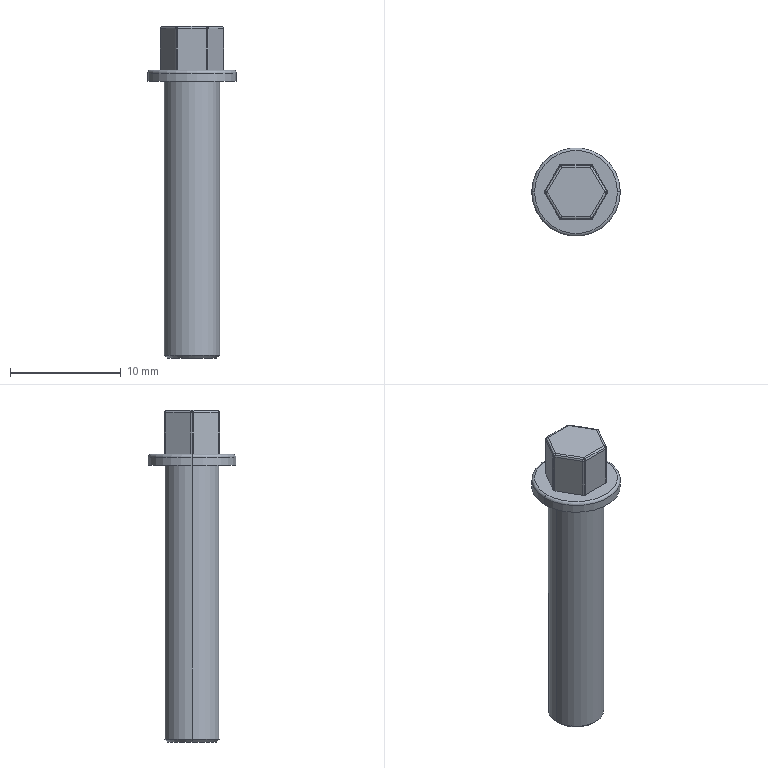Part | SolidWorks | features BaseBody 1 | 1 solid | 54 faces | box 8 x 8 x 30 mm | volume 626.629 mm3 | cylinder 28 | sphere 12 | plane 10 | torus 2 | cone 2 | commonest cylinder face diameters 0.5 x24 5 x2 8 x2
STEP:
#1=CARTESIAN_POINT('',(-1.392,-2.482,4.75));
#2=VERTEX_POINT('',#1);
#3=CARTESIAN_POINT('',(-1.424,-2.467,4.75));
#4=VERTEX_POINT('',#3);
#5=CARTESIAN_POINT('',(-1.299,-2.25,4.75));
#6=DIRECTION('',(0.,0.,-1.));
#7=DIRECTION('',(0.,-1.,0.));
#8=AXIS2_PLACEMENT_3D('',#5,#6,#7);
#9=CIRCLE('',#8,0.25);
#10=EDGE_CURVE('',#2,#4,#9,.T.);
#11=ORIENTED_EDGE('',*,*,#10,.F.);
#12=CARTESIAN_POINT('',(-1.379,-2.296,4.982));
#13=VERTEX_POINT('',#12);
#14=CARTESIAN_POINT('',(-1.299,-2.25,4.75));
#15=DIRECTION('',(-0.9014,0.3603,-0.2402));
#16=DIRECTION('',(-0.3712,-0.9286,0.));
#17=AXIS2_PLACEMENT_3D('',#14,#15,#16);
#18=CIRCLE('',#17,0.25);
#19=EDGE_CURVE('',#2,#13,#18,.T.);
#20=ORIENTED_EDGE('',*,*,#19,.T.);
#21=CARTESIAN_POINT('',(-1.452,-2.338,4.927));
#22=VERTEX_POINT('',#21);
#23=CARTESIAN_POINT('',(-1.299,-2.25,4.75));
#24=DIRECTION('',(-0.5,0.866,0.));
#25=DIRECTION('',(-0.866,-0.5,0.));
#26=AXIS2_PLACEMENT_3D('',#23,#24,#25);
#27=CIRCLE('',#26,0.25);
#28=EDGE_CURVE('',#22,#13,#27,.T.);
#29=ORIENTED_EDGE('',*,*,#28,.F.);
#30=CARTESIAN_POINT('',(-1.516,-2.375,4.75));
#31=VERTEX_POINT('',#30);
#32=CARTESIAN_POINT('',(-1.299,-2.25,4.75));
#33=DIRECTION('',(-0.5,0.866,0.));
#34=DIRECTION('',(-0.866,-0.5,0.));
#35=AXIS2_PLACEMENT_3D('',#32,#33,#34);
#36=CIRCLE('',#35,0.25);
#37=EDGE_CURVE('',#31,#22,#36,.T.);
#38=ORIENTED_EDGE('',*,*,#37,.F.);
#39=CARTESIAN_POINT('',(-1.299,-2.25,4.75));
#40=DIRECTION('',(0.,0.,-1.));
#41=DIRECTION('',(0.,-1.,0.));
#42=AXIS2_PLACEMENT_3D('',#39,#40,#41);
#43=CIRCLE('',#42,0.25);
#44=EDGE_CURVE('',#4,#31,#43,.T.);
#45=ORIENTED_EDGE('',*,*,#44,.F.);
#46=EDGE_LOOP('',(#11,#20,#29,#38,#45));
#47=FACE_OUTER_BOUND('',#46,.T.);
#48=CARTESIAN_POINT('',(-1.299,-2.25,4.75));
#49=DIRECTION('',(0.9014,-0.3603,0.2402));
#50=DIRECTION('',(-0.433,-0.75,0.5));
#51=AXIS2_PLACEMENT_3D('',#48,#49,#50);
#52=SPHERICAL_SURFACE('',#51,0.25);
#53=ADVANCED_FACE('',(#47),#52,.T.);
#54=CARTESIAN_POINT('',(-1.299,-2.5,4.75));
#55=VERTEX_POINT('',#54);
#56=CARTESIAN_POINT('',(-1.299,-2.25,4.75));
#57=DIRECTION('',(0.,0.,-1.));
#58=DIRECTION('',(0.,-1.,0.));
#59=AXIS2_PLACEMENT_3D('',#56,#57,#58);
#60=CIRCLE('',#59,0.25);
#61=EDGE_CURVE('',#55,#2,#60,.T.);
#62=ORIENTED_EDGE('',*,*,#61,.T.);
#63=ORIENTED_EDGE('',*,*,#10,.T.);
#64=CARTESIAN_POINT('',(-1.424,-2.467,1.));
#65=VERTEX_POINT('',#64);
#66=CARTESIAN_POINT('',(-1.424,-2.467,1.));
#67=DIRECTION('',(0.,0.,-1.));
#68=VECTOR('',#67,1000.);
#69=LINE('',#66,#68);
#70=EDGE_CURVE('',#4,#65,#69,.T.);
#71=ORIENTED_EDGE('',*,*,#70,.T.);
#72=CARTESIAN_POINT('',(-1.299,-2.5,1.));
#73=VERTEX_POINT('',#72);
#74=CARTESIAN_POINT('',(-1.299,-2.25,1.));
#75=DIRECTION('',(0.,0.,1.));
#76=DIRECTION('',(-0.5,-0.866,0.));
#77=AXIS2_PLACEMENT_3D('',#74,#75,#76);
#78=CIRCLE('',#77,0.25);
#79=EDGE_CURVE('',#65,#73,#78,.T.);
#80=ORIENTED_EDGE('',*,*,#79,.T.);
#81=CARTESIAN_POINT('',(-1.299,-2.5,1.));
#82=DIRECTION('',(0.,0.,1.));
#83=VECTOR('',#82,1000.);
#84=LINE('',#81,#83);
#85=EDGE_CURVE('',#73,#55,#84,.T.);
#86=ORIENTED_EDGE('',*,*,#85,.T.);
#87=EDGE_LOOP('',(#62,#63,#71,#80,#86));
#88=FACE_OUTER_BOUND('',#87,.T.);
#89=CARTESIAN_POINT('',(-1.299,-2.25,1.));
#90=DIRECTION('',(0.,0.,-1.));
#91=DIRECTION('',(-0.5,-0.866,0.));
#92=AXIS2_PLACEMENT_3D('',#89,#90,#91);
#93=CYLINDRICAL_SURFACE('',#92,0.25);
#94=ADVANCED_FACE('',(#88),#93,.T.);
#95=CARTESIAN_POINT('',(1.392,-2.482,4.75));
#96=VERTEX_POINT('',#95);
#97=CARTESIAN_POINT('',(1.299,-2.5,4.75));
#98=VERTEX_POINT('',#97);
#99=CARTESIAN_POINT('',(1.299,-2.25,4.75));
#100=DIRECTION('',(0.,0.,-1.));
#101=DIRECTION('',(0.866,-0.5,0.));
#102=AXIS2_PLACEMENT_3D('',#99,#100,#101);
#103=CIRCLE('',#102,0.25);
#104=EDGE_CURVE('',#96,#98,#103,.T.);
#105=ORIENTED_EDGE('',*,*,#104,.F.);
#106=CARTESIAN_POINT('',(1.379,-2.296,4.982));
#107=VERTEX_POINT('',#106);
#108=CARTESIAN_POINT('',(1.299,-2.25,4.75));
#109=DIRECTION('',(-0.9014,-0.3603,0.2402));
#110=DIRECTION('',(0.3712,-0.9286,0.));
#111=AXIS2_PLACEMENT_3D('',#108,#109,#110);
#112=CIRCLE('',#111,0.25);
#113=EDGE_CURVE('',#96,#107,#112,.T.);
#114=ORIENTED_EDGE('',*,*,#113,.T.);
#115=CARTESIAN_POINT('',(1.299,-2.25,5.));
#116=VERTEX_POINT('',#115);
#117=CARTESIAN_POINT('',(1.299,-2.25,4.75));
#118=DIRECTION('',(0.5,0.866,0.));
#119=DIRECTION('',(0.,0.,1.));
#120=AXIS2_PLACEMENT_3D('',#117,#118,#119);
#121=CIRCLE('',#120,0.25);
#122=EDGE_CURVE('',#116,#107,#121,.T.);
#123=ORIENTED_EDGE('',*,*,#122,.F.);
#124=CARTESIAN_POINT('',(1.299,-2.427,4.927));
#125=VERTEX_POINT('',#124);
#126=CARTESIAN_POINT('',(1.299,-2.25,4.75));
#127=DIRECTION('',(-1.,0.,0.));
#128=DIRECTION('',(0.,-1.,0.));
#129=AXIS2_PLACEMENT_3D('',#126,#127,#128);
#130=CIRCLE('',#129,0.25);
#131=EDGE_CURVE('',#125,#116,#130,.T.);
#132=ORIENTED_EDGE('',*,*,#131,.F.);
#133=CARTESIAN_POINT('',(1.299,-2.25,4.75));
#134=DIRECTION('',(-1.,0.,0.));
#135=DIRECTION('',(0.,-1.,0.));
#136=AXIS2_PLACEMENT_3D('',#133,#134,#135);
#137=CIRCLE('',#136,0.25);
#138=EDGE_CURVE('',#98,#125,#137,.T.);
#139=ORIENTED_EDGE('',*,*,#138,.F.);
#140=EDGE_LOOP('',(#105,#114,#123,#132,#139));
#141=FACE_OUTER_BOUND('',#140,.T.);
#142=CARTESIAN_POINT('',(1.299,-2.25,4.75));
#143=DIRECTION('',(0.9014,0.3603,-0.2402));
#144=DIRECTION('',(0.433,-0.75,0.5));
#145=AXIS2_PLACEMENT_3D('',#142,#143,#144);
#146=SPHERICAL_SURFACE('',#145,0.25);
#147=ADVANCED_FACE('',(#141),#146,.T.);
#148=CARTESIAN_POINT('',(1.516,-2.375,4.75));
#149=VERTEX_POINT('',#148);
#150=CARTESIAN_POINT('',(1.424,-2.467,4.75));
#151=VERTEX_POINT('',#150);
#152=CARTESIAN_POINT('',(1.299,-2.25,4.75));
#153=DIRECTION('',(0.,0.,-1.));
#154=DIRECTION('',(0.866,-0.5,0.));
#155=AXIS2_PLACEMENT_3D('',#152,#153,#154);
#156=CIRCLE('',#155,0.25);
#157=EDGE_CURVE('',#149,#151,#156,.T.);
#158=ORIENTED_EDGE('',*,*,#157,.T.);
#159=CARTESIAN_POINT('',(1.424,-2.467,1.));
#160=VERTEX_POINT('',#159);
#161=CARTESIAN_POINT('',(1.424,-2.467,1.));
#162=DIRECTION('',(0.,0.,-1.));
#163=VECTOR('',#162,1000.);
#164=LINE('',#161,#163);
#165=EDGE_CURVE('',#151,#160,#164,.T.);
#166=ORIENTED_EDGE('',*,*,#165,.T.);
#167=CARTESIAN_POINT('',(1.516,-2.375,1.));
#168=VERTEX_POINT('',#167);
#169=CARTESIAN_POINT('',(1.299,-2.25,1.));
#170=DIRECTION('',(0.,0.,1.));
#171=DIRECTION('',(0.5,-0.866,0.));
#172=AXIS2_PLACEMENT_3D('',#169,#170,#171);
#173=CIRCLE('',#172,0.25);
#174=EDGE_CURVE('',#160,#168,#173,.T.);
#175=ORIENTED_EDGE('',*,*,#174,.T.);
#176=CARTESIAN_POINT('',(1.516,-2.375,1.));
#177=DIRECTION('',(0.,0.,1.));
#178=VECTOR('',#177,1000.);
#179=LINE('',#176,#178);
#180=EDGE_CURVE('',#168,#149,#179,.T.);
#181=ORIENTED_EDGE('',*,*,#180,.T.);
#182=EDGE_LOOP('',(#158,#166,#175,#181));
#183=FACE_OUTER_BOUND('',#182,.T.);
#184=CARTESIAN_POINT('',(1.299,-2.25,1.));
#185=DIRECTION('',(0.,0.,-1.));
#186=DIRECTION('',(0.5,-0.866,0.));
#187=AXIS2_PLACEMENT_3D('',#184,#185,#186);
#188=CYLINDRICAL_SURFACE('',#187,0.25);
#189=ADVANCED_FACE('',(#183),#188,.T.);
#190=CARTESIAN_POINT('',(-2.792,-0.1118,4.862));
#191=VERTEX_POINT('',#190);
#192=CARTESIAN_POINT('',(-2.815,-0.125,4.75));
#193=VERTEX_POINT('',#192);
#194=CARTESIAN_POINT('',(-2.598,0.,4.75));
#195=DIRECTION('',(0.5,-0.866,0.));
#196=DIRECTION('',(0.,0.,1.));
#197=AXIS2_PLACEMENT_3D('',#194,#195,#196);
#198=CIRCLE('',#197,0.25);
#199=EDGE_CURVE('',#191,#193,#198,.T.);
#200=ORIENTED_EDGE('',*,*,#199,.F.);
#201=CARTESIAN_POINT('',(-2.792,0.1118,4.862));
#202=VERTEX_POINT('',#201);
#203=CARTESIAN_POINT('',(-2.598,0.,4.75));
#204=DIRECTION('',(-0.5,0.,-0.866));
#205=DIRECTION('',(-0.866,0.,0.5));
#206=AXIS2_PLACEMENT_3D('',#203,#204,#205);
#207=CIRCLE('',#206,0.25);
#208=EDGE_CURVE('',#191,#202,#207,.T.);
#209=ORIENTED_EDGE('',*,*,#208,.T.);
#210=CARTESIAN_POINT('',(-2.815,0.125,4.75));
#211=VERTEX_POINT('',#210);
#212=CARTESIAN_POINT('',(-2.598,0.,4.75));
#213=DIRECTION('',(0.5,0.866,0.));
#214=DIRECTION('',(-0.866,0.5,0.));
#215=AXIS2_PLACEMENT_3D('',#212,#213,#214);
#216=CIRCLE('',#215,0.25);
#217=EDGE_CURVE('',#211,#202,#216,.T.);
#218=ORIENTED_EDGE('',*,*,#217,.F.);
#219=CARTESIAN_POINT('',(-2.848,0.,4.75));
#220=VERTEX_POINT('',#219);
#221=CARTESIAN_POINT('',(-2.598,0.,4.75));
#222=DIRECTION('',(0.,0.,-1.));
#223=DIRECTION('',(-0.866,-0.5,0.));
#224=AXIS2_PLACEMENT_3D('',#221,#222,#223);
#225=CIRCLE('',#224,0.25);
#226=EDGE_CURVE('',#220,#211,#225,.T.);
#227=ORIENTED_EDGE('',*,*,#226,.F.);
#228=CARTESIAN_POINT('',(-2.598,0.,4.75));
#229=DIRECTION('',(0.,0.,-1.));
#230=DIRECTION('',(-0.866,-0.5,0.));
#231=AXIS2_PLACEMENT_3D('',#228,#229,#230);
#232=CIRCLE('',#231,0.25);
#233=EDGE_CURVE('',#193,#220,#232,.T.);
#234=ORIENTED_EDGE('',*,*,#233,.F.);
#235=EDGE_LOOP('',(#200,#209,#218,#227,#234));
#236=FACE_OUTER_BOUND('',#235,.T.);
#237=CARTESIAN_POINT('',(-2.598,0.,4.75));
#238=DIRECTION('',(0.5,0.,0.866));
#239=DIRECTION('',(-0.866,0.,0.5));
#240=AXIS2_PLACEMENT_3D('',#237,#238,#239);
#241=SPHERICAL_SURFACE('',#240,0.25);
#242=ADVANCED_FACE('',(#236),#241,.T.);
#243=ORIENTED_EDGE('',*,*,#233,.T.);
#244=CARTESIAN_POINT('',(-2.848,0.,1.));
#245=VERTEX_POINT('',#244);
#246=CARTESIAN_POINT('',(-2.848,0.,1.));
#247=DIRECTION('',(0.,0.,-1.));
#248=VECTOR('',#247,1000.);
#249=LINE('',#246,#248);
#250=EDGE_CURVE('',#220,#245,#249,.T.);
#251=ORIENTED_EDGE('',*,*,#250,.T.);
#252=CARTESIAN_POINT('',(-2.815,-0.125,1.));
#253=VERTEX_POINT('',#252);
#254=CARTESIAN_POINT('',(-2.598,0.,1.));
#255=DIRECTION('',(0.,0.,1.));
#256=DIRECTION('',(-1.,0.,0.));
#257=AXIS2_PLACEMENT_3D('',#254,#255,#256);
#258=CIRCLE('',#257,0.25);
#259=EDGE_CURVE('',#245,#253,#258,.T.);
#260=ORIENTED_EDGE('',*,*,#259,.T.);
#261=CARTESIAN_POINT('',(-2.815,-0.125,1.));
#262=DIRECTION('',(0.,0.,1.));
#263=VECTOR('',#262,1000.);
#264=LINE('',#261,#263);
#265=EDGE_CURVE('',#253,#193,#264,.T.);
#266=ORIENTED_EDGE('',*,*,#265,.T.);
#267=EDGE_LOOP('',(#243,#251,#260,#266));
#268=FACE_OUTER_BOUND('',#267,.T.);
#269=CARTESIAN_POINT('',(-2.598,0.,1.));
#270=DIRECTION('',(0.,0.,-1.));
#271=DIRECTION('',(-1.,0.,0.));
#272=AXIS2_PLACEMENT_3D('',#269,#270,#271);
#273=CYLINDRICAL_SURFACE('',#272,0.25);
#274=ADVANCED_FACE('',(#268),#273,.T.);
#275=ORIENTED_EDGE('',*,*,#37,.T.);
#276=CARTESIAN_POINT('',(-2.751,-0.08839,4.927));
#277=VERTEX_POINT('',#276);
#278=CARTESIAN_POINT('',(-2.462,-0.5884,4.927));
#279=DIRECTION('',(-0.5,0.866,0.));
#280=VECTOR('',#279,1000.);
#281=LINE('',#278,#280);
#282=EDGE_CURVE('',#22,#277,#281,.T.);
#283=ORIENTED_EDGE('',*,*,#282,.T.);
#284=CARTESIAN_POINT('',(-2.598,0.,4.75));
#285=DIRECTION('',(0.5,-0.866,0.));
#286=DIRECTION('',(0.,0.,1.));
#287=AXIS2_PLACEMENT_3D('',#284,#285,#286);
#288=CIRCLE('',#287,0.25);
#289=EDGE_CURVE('',#277,#191,#288,.T.);
#290=ORIENTED_EDGE('',*,*,#289,.T.);
#291=ORIENTED_EDGE('',*,*,#199,.T.);
#292=CARTESIAN_POINT('',(-2.526,-0.625,4.75));
#293=DIRECTION('',(0.5,-0.866,0.));
#294=VECTOR('',#293,1000.);
#295=LINE('',#292,#294);
#296=EDGE_CURVE('',#193,#31,#295,.T.);
#297=ORIENTED_EDGE('',*,*,#296,.T.);
#298=EDGE_LOOP('',(#275,#283,#290,#291,#297));
#299=FACE_OUTER_BOUND('',#298,.T.);
#300=CARTESIAN_POINT('',(-2.309,-0.5,4.75));
#301=DIRECTION('',(-0.5,0.866,0.));
#302=DIRECTION('',(-0.6124,-0.3536,0.7071));
#303=AXIS2_PLACEMENT_3D('',#300,#301,#302);
#304=CYLINDRICAL_SURFACE('',#303,0.25);
#305=ADVANCED_FACE('',(#299),#304,.T.);
#306=CARTESIAN_POINT('',(2.792,0.1118,4.862));
#307=VERTEX_POINT('',#306);
#308=CARTESIAN_POINT('',(2.815,0.125,4.75));
#309=VERTEX_POINT('',#308);
#310=CARTESIAN_POINT('',(2.598,0.,4.75));
#311=DIRECTION('',(-0.5,0.866,0.));
#312=DIRECTION('',(0.,0.,1.));
#313=AXIS2_PLACEMENT_3D('',#310,#311,#312);
#314=CIRCLE('',#313,0.25);
#315=EDGE_CURVE('',#307,#309,#314,.T.);
#316=ORIENTED_EDGE('',*,*,#315,.F.);
#317=CARTESIAN_POINT('',(2.792,-0.1118,4.862));
#318=VERTEX_POINT('',#317);
#319=CARTESIAN_POINT('',(2.598,0.,4.75));
#320=DIRECTION('',(0.5,0.,-0.866));
#321=DIRECTION('',(-0.866,0.,-0.5));
#322=AXIS2_PLACEMENT_3D('',#319,#320,#321);
#323=CIRCLE('',#322,0.25);
#324=EDGE_CURVE('',#307,#318,#323,.T.);
#325=ORIENTED_EDGE('',*,*,#324,.T.);
#326=CARTESIAN_POINT('',(2.815,-0.125,4.75));
#327=VERTEX_POINT('',#326);
#328=CARTESIAN_POINT('',(2.598,0.,4.75));
#329=DIRECTION('',(-0.5,-0.866,0.));
#330=DIRECTION('',(0.866,-0.5,0.));
#331=AXIS2_PLACEMENT_3D('',#328,#329,#330);
#332=CIRCLE('',#331,0.25);
#333=EDGE_CURVE('',#327,#318,#332,.T.);
#334=ORIENTED_EDGE('',*,*,#333,.F.);
#335=CARTESIAN_POINT('',(2.848,0.,4.75));
#336=VERTEX_POINT('',#335);
#337=CARTESIAN_POINT('',(2.598,0.,4.75));
#338=DIRECTION('',(0.,0.,-1.));
#339=DIRECTION('',(0.866,0.5,0.));
#340=AXIS2_PLACEMENT_3D('',#337,#338,#339);
#341=CIRCLE('',#340,0.25);
#342=EDGE_CURVE('',#336,#327,#341,.T.);
#343=ORIENTED_EDGE('',*,*,#342,.F.);
#344=CARTESIAN_POINT('',(2.598,0.,4.75));
#345=DIRECTION('',(0.,0.,-1.));
#346=DIRECTION('',(0.866,0.5,0.));
#347=AXIS2_PLACEMENT_3D('',#344,#345,#346);
#348=CIRCLE('',#347,0.25);
#349=EDGE_CURVE('',#309,#336,#348,.T.);
#350=ORIENTED_EDGE('',*,*,#349,.F.);
#351=EDGE_LOOP('',(#316,#325,#334,#343,#350));
#352=FACE_OUTER_BOUND('',#351,.T.);
#353=CARTESIAN_POINT('',(2.598,0.,4.75));
#354=DIRECTION('',(-0.5,0.,0.866));
#355=DIRECTION('',(0.866,0.,0.5));
#356=AXIS2_PLACEMENT_3D('',#353,#354,#355);
#357=SPHERICAL_SURFACE('',#356,0.25);
#358=ADVANCED_FACE('',(#352),#357,.T.);
#359=ORIENTED_EDGE('',*,*,#349,.T.);
#360=CARTESIAN_POINT('',(2.848,0.,1.));
#361=VERTEX_POINT('',#360);
#362=CARTESIAN_POINT('',(2.848,0.,1.));
#363=DIRECTION('',(0.,0.,-1.));
#364=VECTOR('',#363,1000.);
#365=LINE('',#362,#364);
#366=EDGE_CURVE('',#336,#361,#365,.T.);
#367=ORIENTED_EDGE('',*,*,#366,.T.);
#368=CARTESIAN_POINT('',(2.815,0.125,1.));
#369=VERTEX_POINT('',#368);
#370=CARTESIAN_POINT('',(2.598,0.,1.));
#371=DIRECTION('',(0.,0.,1.));
#372=DIRECTION('',(1.,0.,0.));
#373=AXIS2_PLACEMENT_3D('',#370,#371,#372);
#374=CIRCLE('',#373,0.25);
#375=EDGE_CURVE('',#361,#369,#374,.T.);
#376=ORIENTED_EDGE('',*,*,#375,.T.);
#377=CARTESIAN_POINT('',(2.815,0.125,1.));
#378=DIRECTION('',(0.,0.,1.));
#379=VECTOR('',#378,1000.);
#380=LINE('',#377,#379);
#381=EDGE_CURVE('',#369,#309,#380,.T.);
#382=ORIENTED_EDGE('',*,*,#381,.T.);
#383=EDGE_LOOP('',(#359,#367,#376,#382));
#384=FACE_OUTER_BOUND('',#383,.T.);
#385=CARTESIAN_POINT('',(2.598,0.,1.));
#386=DIRECTION('',(0.,0.,-1.));
#387=DIRECTION('',(1.,0.,0.));
#388=AXIS2_PLACEMENT_3D('',#385,#386,#387);
#389=CYLINDRICAL_SURFACE('',#388,0.25);
#390=ADVANCED_FACE('',(#384),#389,.T.);
#391=CARTESIAN_POINT('',(-1.379,2.296,4.982));
#392=VERTEX_POINT('',#391);
#393=CARTESIAN_POINT('',(-1.452,2.338,4.927));
#394=VERTEX_POINT('',#393);
#395=CARTESIAN_POINT('',(-1.299,2.25,4.75));
#396=DIRECTION('',(-0.5,-0.866,0.));
#397=DIRECTION('',(0.,0.,1.));
#398=AXIS2_PLACEMENT_3D('',#395,#396,#397);
#399=CIRCLE('',#398,0.25);
#400=EDGE_CURVE('',#392,#394,#399,.T.);
#401=ORIENTED_EDGE('',*,*,#400,.F.);
#402=CARTESIAN_POINT('',(-1.392,2.482,4.75));
#403=VERTEX_POINT('',#402);
#404=CARTESIAN_POINT('',(-1.299,2.25,4.75));
#405=DIRECTION('',(-0.9014,-0.3603,-0.2402));
#406=DIRECTION('',(0.3712,-0.9286,0.));
#407=AXIS2_PLACEMENT_3D('',#404,#405,#406);
#408=CIRCLE('',#407,0.25);
#409=EDGE_CURVE('',#392,#403,#408,.T.);
#410=ORIENTED_EDGE('',*,*,#409,.T.);
#411=CARTESIAN_POINT('',(-1.424,2.467,4.75));
#412=VERTEX_POINT('',#411);
#413=CARTESIAN_POINT('',(-1.299,2.25,4.75));
#414=DIRECTION('',(0.,0.,-1.));
#415=DIRECTION('',(-0.866,0.5,0.));
#416=AXIS2_PLACEMENT_3D('',#413,#414,#415);
#417=CIRCLE('',#416,0.25);
#418=EDGE_CURVE('',#412,#403,#417,.T.);
#419=ORIENTED_EDGE('',*,*,#418,.F.);
#420=CARTESIAN_POINT('',(-1.516,2.375,4.75));
#421=VERTEX_POINT('',#420);
#422=CARTESIAN_POINT('',(-1.299,2.25,4.75));
#423=DIRECTION('',(0.,0.,-1.));
#424=DIRECTION('',(-0.866,0.5,0.));
#425=AXIS2_PLACEMENT_3D('',#422,#423,#424);
#426=CIRCLE('',#425,0.25);
#427=EDGE_CURVE('',#421,#412,#426,.T.);
#428=ORIENTED_EDGE('',*,*,#427,.F.);
#429=CARTESIAN_POINT('',(-1.299,2.25,4.75));
#430=DIRECTION('',(-0.5,-0.866,0.));
#431=DIRECTION('',(0.,0.,1.));
#432=AXIS2_PLACEMENT_3D('',#429,#430,#431);
#433=CIRCLE('',#432,0.25);
#434=EDGE_CURVE('',#394,#421,#433,.T.);
#435=ORIENTED_EDGE('',*,*,#434,.F.);
#436=EDGE_LOOP('',(#401,#410,#419,#428,#435));
#437=FACE_OUTER_BOUND('',#436,.T.);
#438=CARTESIAN_POINT('',(-1.299,2.25,4.75));
#439=DIRECTION('',(0.9014,0.3603,0.2402));
#440=DIRECTION('',(-0.433,0.75,0.5));
#441=AXIS2_PLACEMENT_3D('',#438,#439,#440);
#442=SPHERICAL_SURFACE('',#441,0.25);
#443=ADVANCED_FACE('',(#437),#442,.T.);
#444=ORIENTED_EDGE('',*,*,#427,.T.);
#445=CARTESIAN_POINT('',(-1.424,2.467,1.));
#446=VERTEX_POINT('',#445);
#447=CARTESIAN_POINT('',(-1.424,2.467,1.));
#448=DIRECTION('',(0.,0.,-1.));
#449=VECTOR('',#448,1000.);
#450=LINE('',#447,#449);
#451=EDGE_CURVE('',#412,#446,#450,.T.);
#452=ORIENTED_EDGE('',*,*,#451,.T.);
#453=CARTESIAN_POINT('',(-1.516,2.375,1.));
#454=VERTEX_POINT('',#453);
#455=CARTESIAN_POINT('',(-1.299,2.25,1.));
#456=DIRECTION('',(0.,0.,1.));
#457=DIRECTION('',(-0.5,0.866,0.));
#458=AXIS2_PLACEMENT_3D('',#455,#456,#457);
#459=CIRCLE('',#458,0.25);
#460=EDGE_CURVE('',#446,#454,#459,.T.);
#461=ORIENTED_EDGE('',*,*,#460,.T.);
#462=CARTESIAN_POINT('',(-1.516,2.375,1.));
#463=DIRECTION('',(0.,0.,1.));
#464=VECTOR('',#463,1000.);
#465=LINE('',#462,#464);
#466=EDGE_CURVE('',#454,#421,#465,.T.);
#467=ORIENTED_EDGE('',*,*,#466,.T.);
#468=EDGE_LOOP('',(#444,#452,#461,#467));
#469=FACE_OUTER_BOUND('',#468,.T.);
#470=CARTESIAN_POINT('',(-1.299,2.25,1.));
#471=DIRECTION('',(0.,0.,-1.));
#472=DIRECTION('',(-0.5,0.866,0.));
#473=AXIS2_PLACEMENT_3D('',#470,#471,#472);
#474=CYLINDRICAL_SURFACE('',#473,0.25);
#475=ADVANCED_FACE('',(#469),#474,.T.);
#476=ORIENTED_EDGE('',*,*,#217,.T.);
#477=CARTESIAN_POINT('',(-2.751,0.08839,4.927));
#478=VERTEX_POINT('',#477);
#479=CARTESIAN_POINT('',(-2.598,0.,4.75));
#480=DIRECTION('',(0.5,0.866,0.));
#481=DIRECTION('',(-0.866,0.5,0.));
#482=AXIS2_PLACEMENT_3D('',#479,#480,#481);
#483=CIRCLE('',#482,0.25);
#484=EDGE_CURVE('',#202,#478,#483,.T.);
#485=ORIENTED_EDGE('',*,*,#484,.T.);
#486=CARTESIAN_POINT('',(-1.741,1.838,4.927));
#487=DIRECTION('',(0.5,0.866,0.));
#488=VECTOR('',#487,1000.);
#489=LINE('',#486,#488);
#490=EDGE_CURVE('',#478,#394,#489,.T.);
#491=ORIENTED_EDGE('',*,*,#490,.T.);
#492=ORIENTED_EDGE('',*,*,#434,.T.);
#493=CARTESIAN_POINT('',(-1.804,1.875,4.75));
#494=DIRECTION('',(-0.5,-0.866,0.));
#495=VECTOR('',#494,1000.);
#496=LINE('',#493,#495);
#497=EDGE_CURVE('',#421,#211,#496,.T.);
#498=ORIENTED_EDGE('',*,*,#497,.T.);
#499=EDGE_LOOP('',(#476,#485,#491,#492,#498));
#500=FACE_OUTER_BOUND('',#499,.T.);
#501=CARTESIAN_POINT('',(-1.588,1.75,4.75));
#502=DIRECTION('',(0.5,0.866,0.));
#503=DIRECTION('',(-0.6124,0.3536,0.7071));
#504=AXIS2_PLACEMENT_3D('',#501,#502,#503);
#505=CYLINDRICAL_SURFACE('',#504,0.25);
#506=ADVANCED_FACE('',(#500),#505,.T.);
#507=CARTESIAN_POINT('',(1.379,2.296,4.982));
#508=VERTEX_POINT('',#507);
#509=CARTESIAN_POINT('',(1.299,2.25,5.));
#510=VERTEX_POINT('',#509);
#511=CARTESIAN_POINT('',(1.299,2.25,4.75));
#512=DIRECTION('',(0.5,-0.866,0.));
#513=DIRECTION('',(0.866,0.5,0.));
#514=AXIS2_PLACEMENT_3D('',#511,#512,#513);
#515=CIRCLE('',#514,0.25);
#516=EDGE_CURVE('',#508,#510,#515,.T.);
#517=ORIENTED_EDGE('',*,*,#516,.F.);
#518=CARTESIAN_POINT('',(1.392,2.482,4.75));
#519=VERTEX_POINT('',#518);
#520=CARTESIAN_POINT('',(1.299,2.25,4.75));
#521=DIRECTION('',(-0.9014,0.3603,0.2402));
#522=DIRECTION('',(-0.3712,-0.9286,0.));
#523=AXIS2_PLACEMENT_3D('',#520,#521,#522);
#524=CIRCLE('',#523,0.25);
#525=EDGE_CURVE('',#508,#519,#524,.T.);
#526=ORIENTED_EDGE('',*,*,#525,.T.);
#527=CARTESIAN_POINT('',(1.299,2.5,4.75));
#528=VERTEX_POINT('',#527);
#529=CARTESIAN_POINT('',(1.299,2.25,4.75));
#530=DIRECTION('',(0.,0.,-1.));
#531=DIRECTION('',(0.,1.,0.));
#532=AXIS2_PLACEMENT_3D('',#529,#530,#531);
#533=CIRCLE('',#532,0.25);
#534=EDGE_CURVE('',#528,#519,#533,.T.);
#535=ORIENTED_EDGE('',*,*,#534,.F.);
#536=CARTESIAN_POINT('',(1.299,2.427,4.927));
#537=VERTEX_POINT('',#536);
#538=CARTESIAN_POINT('',(1.299,2.25,4.75));
#539=DIRECTION('',(-1.,0.,0.));
#540=DIRECTION('',(0.,0.,1.));
#541=AXIS2_PLACEMENT_3D('',#538,#539,#540);
#542=CIRCLE('',#541,0.25);
#543=EDGE_CURVE('',#537,#528,#542,.T.);
#544=ORIENTED_EDGE('',*,*,#543,.F.);
#545=CARTESIAN_POINT('',(1.299,2.25,4.75));
#546=DIRECTION('',(-1.,0.,0.));
#547=DIRECTION('',(0.,0.,1.));
#548=AXIS2_PLACEMENT_3D('',#545,#546,#547);
#549=CIRCLE('',#548,0.25);
#550=EDGE_CURVE('',#510,#537,#549,.T.);
#551=ORIENTED_EDGE('',*,*,#550,.F.);
#552=EDGE_LOOP('',(#517,#526,#535,#544,#551));
#553=FACE_OUTER_BOUND('',#552,.T.);
#554=CARTESIAN_POINT('',(1.299,2.25,4.75));
#555=DIRECTION('',(0.9014,-0.3603,-0.2402));
#556=DIRECTION('',(0.433,0.75,0.5));
#557=AXIS2_PLACEMENT_3D('',#554,#555,#556);
#558=SPHERICAL_SURFACE('',#557,0.25);
#559=ADVANCED_FACE('',(#553),#558,.T.);
#560=ORIENTED_EDGE('',*,*,#534,.T.);
#561=CARTESIAN_POINT('',(1.424,2.467,4.75));
#562=VERTEX_POINT('',#561);
#563=CARTESIAN_POINT('',(1.299,2.25,4.75));
#564=DIRECTION('',(0.,0.,-1.));
#565=DIRECTION('',(0.,1.,0.));
#566=AXIS2_PLACEMENT_3D('',#563,#564,#565);
#567=CIRCLE('',#566,0.25);
#568=EDGE_CURVE('',#519,#562,#567,.T.);
#569=ORIENTED_EDGE('',*,*,#568,.T.);
#570=CARTESIAN_POINT('',(1.424,2.467,1.));
#571=VERTEX_POINT('',#570);
#572=CARTESIAN_POINT('',(1.424,2.467,1.));
#573=DIRECTION('',(0.,0.,-1.));
#574=VECTOR('',#573,1000.);
#575=LINE('',#572,#574);
#576=EDGE_CURVE('',#562,#571,#575,.T.);
#577=ORIENTED_EDGE('',*,*,#576,.T.);
#578=CARTESIAN_POINT('',(1.299,2.5,1.));
#579=VERTEX_POINT('',#578);
#580=CARTESIAN_POINT('',(1.299,2.25,1.));
#581=DIRECTION('',(0.,0.,1.));
#582=DIRECTION('',(0.5,0.866,0.));
#583=AXIS2_PLACEMENT_3D('',#580,#581,#582);
#584=CIRCLE('',#583,0.25);
#585=EDGE_CURVE('',#571,#579,#584,.T.);
#586=ORIENTED_EDGE('',*,*,#585,.T.);
#587=CARTESIAN_POINT('',(1.299,2.5,1.));
#588=DIRECTION('',(0.,0.,1.));
#589=VECTOR('',#588,1000.);
#590=LINE('',#587,#589);
#591=EDGE_CURVE('',#579,#528,#590,.T.);
#592=ORIENTED_EDGE('',*,*,#591,.T.);
#593=EDGE_LOOP('',(#560,#569,#577,#586,#592));
#594=FACE_OUTER_BOUND('',#593,.T.);
#595=CARTESIAN_POINT('',(1.299,2.25,1.));
#596=DIRECTION('',(0.,0.,-1.));
#597=DIRECTION('',(0.5,0.866,0.));
#598=AXIS2_PLACEMENT_3D('',#595,#596,#597);
#599=CYLINDRICAL_SURFACE('',#598,0.25);
#600=ADVANCED_FACE('',(#594),#599,.T.);
#601=CARTESIAN_POINT('',(-1.299,2.5,4.75));
#602=VERTEX_POINT('',#601);
#603=CARTESIAN_POINT('',(-1.299,2.427,4.927));
#604=VERTEX_POINT('',#603);
#605=CARTESIAN_POINT('',(-1.299,2.25,4.75));
#606=DIRECTION('',(1.,0.,0.));
#607=DIRECTION('',(0.,1.,0.));
#608=AXIS2_PLACEMENT_3D('',#605,#606,#607);
#609=CIRCLE('',#608,0.25);
#610=EDGE_CURVE('',#602,#604,#609,.T.);
#611=ORIENTED_EDGE('',*,*,#610,.T.);
#612=CARTESIAN_POINT('',(0.7217,2.427,4.927));
#613=DIRECTION('',(1.,0.,0.));
#614=VECTOR('',#613,1000.);
#615=LINE('',#612,#614);
#616=EDGE_CURVE('',#604,#537,#615,.T.);
#617=ORIENTED_EDGE('',*,*,#616,.T.);
#618=ORIENTED_EDGE('',*,*,#543,.T.);
#619=CARTESIAN_POINT('',(0.7217,2.5,4.75));
#620=DIRECTION('',(-1.,0.,0.));
#621=VECTOR('',#620,1000.);
#622=LINE('',#619,#621);
#623=EDGE_CURVE('',#528,#602,#622,.T.);
#624=ORIENTED_EDGE('',*,*,#623,.T.);
#625=EDGE_LOOP('',(#611,#617,#618,#624));
#626=FACE_OUTER_BOUND('',#625,.T.);
#627=CARTESIAN_POINT('',(0.7217,2.25,4.75));
#628=DIRECTION('',(1.,0.,0.));
#629=DIRECTION('',(0.,0.7071,0.7071));
#630=AXIS2_PLACEMENT_3D('',#627,#628,#629);
#631=CYLINDRICAL_SURFACE('',#630,0.25);
#632=ADVANCED_FACE('',(#626),#631,.T.);
#633=CARTESIAN_POINT('',(1.516,2.375,4.75));
#634=VERTEX_POINT('',#633);
#635=CARTESIAN_POINT('',(1.452,2.338,4.927));
#636=VERTEX_POINT('',#635);
#637=CARTESIAN_POINT('',(1.299,2.25,4.75));
#638=DIRECTION('',(0.5,-0.866,0.));
#639=DIRECTION('',(0.866,0.5,0.));
#640=AXIS2_PLACEMENT_3D('',#637,#638,#639);
#641=CIRCLE('',#640,0.25);
#642=EDGE_CURVE('',#634,#636,#641,.T.);
#643=ORIENTED_EDGE('',*,*,#642,.T.);
#644=CARTESIAN_POINT('',(2.751,0.08839,4.927));
#645=VERTEX_POINT('',#644);
#646=CARTESIAN_POINT('',(2.462,0.5884,4.927));
#647=DIRECTION('',(0.5,-0.866,0.));
#648=VECTOR('',#647,1000.);
#649=LINE('',#646,#648);
#650=EDGE_CURVE('',#636,#645,#649,.T.);
#651=ORIENTED_EDGE('',*,*,#650,.T.);
#652=CARTESIAN_POINT('',(2.598,0.,4.75));
#653=DIRECTION('',(-0.5,0.866,0.));
#654=DIRECTION('',(0.,0.,1.));
#655=AXIS2_PLACEMENT_3D('',#652,#653,#654);
#656=CIRCLE('',#655,0.25);
#657=EDGE_CURVE('',#645,#307,#656,.T.);
#658=ORIENTED_EDGE('',*,*,#657,.T.);
#659=ORIENTED_EDGE('',*,*,#315,.T.);
#660=CARTESIAN_POINT('',(2.526,0.625,4.75));
#661=DIRECTION('',(-0.5,0.866,0.));
#662=VECTOR('',#661,1000.);
#663=LINE('',#660,#662);
#664=EDGE_CURVE('',#309,#634,#663,.T.);
#665=ORIENTED_EDGE('',*,*,#664,.T.);
#666=EDGE_LOOP('',(#643,#651,#658,#659,#665));
#667=FACE_OUTER_BOUND('',#666,.T.);
#668=CARTESIAN_POINT('',(2.309,0.5,4.75));
#669=DIRECTION('',(0.5,-0.866,0.));
#670=DIRECTION('',(0.6124,0.3536,0.7071));
#671=AXIS2_PLACEMENT_3D('',#668,#669,#670);
#672=CYLINDRICAL_SURFACE('',#671,0.25);
#673=ADVANCED_FACE('',(#667),#672,.T.);
#674=ORIENTED_EDGE('',*,*,#333,.T.);
#675=CARTESIAN_POINT('',(2.751,-0.08839,4.927));
#676=VERTEX_POINT('',#675);
#677=CARTESIAN_POINT('',(2.598,0.,4.75));
#678=DIRECTION('',(-0.5,-0.866,0.));
#679=DIRECTION('',(0.866,-0.5,0.));
#680=AXIS2_PLACEMENT_3D('',#677,#678,#679);
#681=CIRCLE('',#680,0.25);
#682=EDGE_CURVE('',#318,#676,#681,.T.);
#683=ORIENTED_EDGE('',*,*,#682,.T.);
#684=CARTESIAN_POINT('',(1.452,-2.338,4.927));
#685=VERTEX_POINT('',#684);
#686=CARTESIAN_POINT('',(1.741,-1.838,4.927));
#687=DIRECTION('',(-0.5,-0.866,0.));
#688=VECTOR('',#687,1000.);
#689=LINE('',#686,#688);
#690=EDGE_CURVE('',#676,#685,#689,.T.);
#691=ORIENTED_EDGE('',*,*,#690,.T.);
#692=CARTESIAN_POINT('',(1.299,-2.25,4.75));
#693=DIRECTION('',(0.5,0.866,0.));
#694=DIRECTION('',(0.,0.,1.));
#695=AXIS2_PLACEMENT_3D('',#692,#693,#694);
#696=CIRCLE('',#695,0.25);
#697=EDGE_CURVE('',#685,#149,#696,.T.);
#698=ORIENTED_EDGE('',*,*,#697,.T.);
#699=CARTESIAN_POINT('',(1.804,-1.875,4.75));
#700=DIRECTION('',(0.5,0.866,0.));
#701=VECTOR('',#700,1000.);
#702=LINE('',#699,#701);
#703=EDGE_CURVE('',#149,#327,#702,.T.);
#704=ORIENTED_EDGE('',*,*,#703,.T.);
#705=EDGE_LOOP('',(#674,#683,#691,#698,#704));
#706=FACE_OUTER_BOUND('',#705,.T.);
#707=CARTESIAN_POINT('',(1.588,-1.75,4.75));
#708=DIRECTION('',(-0.5,-0.866,0.));
#709=DIRECTION('',(0.6124,-0.3536,0.7071));
#710=AXIS2_PLACEMENT_3D('',#707,#708,#709);
#711=CYLINDRICAL_SURFACE('',#710,0.25);
#712=ADVANCED_FACE('',(#706),#711,.T.);
#713=ORIENTED_EDGE('',*,*,#138,.T.);
#714=CARTESIAN_POINT('',(-1.299,-2.427,4.927));
#715=VERTEX_POINT('',#714);
#716=CARTESIAN_POINT('',(-0.7217,-2.427,4.927));
#717=DIRECTION('',(-1.,0.,0.));
#718=VECTOR('',#717,1000.);
#719=LINE('',#716,#718);
#720=EDGE_CURVE('',#125,#715,#719,.T.);
#721=ORIENTED_EDGE('',*,*,#720,.T.);
#722=CARTESIAN_POINT('',(-1.299,-2.25,4.75));
#723=DIRECTION('',(1.,0.,0.));
#724=DIRECTION('',(0.,0.,1.));
#725=AXIS2_PLACEMENT_3D('',#722,#723,#724);
#726=CIRCLE('',#725,0.25);
#727=EDGE_CURVE('',#715,#55,#726,.T.);
#728=ORIENTED_EDGE('',*,*,#727,.T.);
#729=CARTESIAN_POINT('',(-0.7217,-2.5,4.75));
#730=DIRECTION('',(1.,0.,0.));
#731=VECTOR('',#730,1000.);
#732=LINE('',#729,#731);
#733=EDGE_CURVE('',#55,#98,#732,.T.);
#734=ORIENTED_EDGE('',*,*,#733,.T.);
#735=EDGE_LOOP('',(#713,#721,#728,#734));
#736=FACE_OUTER_BOUND('',#735,.T.);
#737=CARTESIAN_POINT('',(-0.7217,-2.25,4.75));
#738=DIRECTION('',(-1.,0.,0.));
#739=DIRECTION('',(0.,-0.7071,0.7071));
#740=AXIS2_PLACEMENT_3D('',#737,#738,#739);
#741=CYLINDRICAL_SURFACE('',#740,0.25);
#742=ADVANCED_FACE('',(#736),#741,.T.);
#743=CARTESIAN_POINT('',(4.,0.,0.75));
#744=VERTEX_POINT('',#743);
#745=CARTESIAN_POINT('',(-4.,0.,0.75));
#746=VERTEX_POINT('',#745);
#747=CARTESIAN_POINT('',(0.,0.,0.75));
#748=DIRECTION('',(0.,0.,1.));
#749=DIRECTION('',(-1.,0.,0.));
#750=AXIS2_PLACEMENT_3D('',#747,#748,#749);
#751=CIRCLE('',#750,4.);
#752=EDGE_CURVE('',#744,#746,#751,.T.);
#753=ORIENTED_EDGE('',*,*,#752,.T.);
#754=CARTESIAN_POINT('',(-3.75,0.,1.));
#755=VERTEX_POINT('',#754);
#756=CARTESIAN_POINT('',(-3.75,0.,0.75));
#757=DIRECTION('',(0.,1.,0.));
#758=DIRECTION('',(-1.,0.,0.));
#759=AXIS2_PLACEMENT_3D('',#756,#757,#758);
#760=CIRCLE('',#759,0.25);
#761=EDGE_CURVE('',#746,#755,#760,.T.);
#762=ORIENTED_EDGE('',*,*,#761,.T.);
#763=CARTESIAN_POINT('',(3.75,0.,1.));
#764=VERTEX_POINT('',#763);
#765=CARTESIAN_POINT('',(0.,0.,1.));
#766=DIRECTION('',(0.,0.,-1.));
#767=DIRECTION('',(-1.,0.,0.));
#768=AXIS2_PLACEMENT_3D('',#765,#766,#767);
#769=CIRCLE('',#768,3.75);
#770=EDGE_CURVE('',#755,#764,#769,.T.);
#771=ORIENTED_EDGE('',*,*,#770,.T.);
#772=CARTESIAN_POINT('',(3.75,0.,0.75));
#773=DIRECTION('',(0.,-1.,0.));
#774=DIRECTION('',(0.,0.,-1.));
#775=AXIS2_PLACEMENT_3D('',#772,#773,#774);
#776=CIRCLE('',#775,0.25);
#777=EDGE_CURVE('',#744,#764,#776,.T.);
#778=ORIENTED_EDGE('',*,*,#777,.F.);
#779=EDGE_LOOP('',(#753,#762,#771,#778));
#780=FACE_OUTER_BOUND('',#779,.T.);
#781=CARTESIAN_POINT('',(0.,0.,0.75));
#782=DIRECTION('',(0.,0.,1.));
#783=DIRECTION('',(1.,0.,0.));
#784=AXIS2_PLACEMENT_3D('',#781,#782,#783);
#785=TOROIDAL_SURFACE('',#784,3.75,0.25);
#786=ADVANCED_FACE('',(#780),#785,.T.);
#787=ORIENTED_EDGE('',*,*,#752,.F.);
#788=CARTESIAN_POINT('',(4.,0.,0.));
#789=VERTEX_POINT('',#788);
#790=CARTESIAN_POINT('',(4.,0.,0.));
#791=DIRECTION('',(0.,0.,-1.));
#792=VECTOR('',#791,1000.);
#793=LINE('',#790,#792);
#794=EDGE_CURVE('',#744,#789,#793,.T.);
#795=ORIENTED_EDGE('',*,*,#794,.T.);
#796=CARTESIAN_POINT('',(-4.,0.,0.));
#797=VERTEX_POINT('',#796);
#798=CARTESIAN_POINT('',(0.,0.,0.));
#799=DIRECTION('',(0.,0.,-1.));
#800=DIRECTION('',(-1.,0.,0.));
#801=AXIS2_PLACEMENT_3D('',#798,#799,#800);
#802=CIRCLE('',#801,4.);
#803=EDGE_CURVE('',#797,#789,#802,.T.);
#804=ORIENTED_EDGE('',*,*,#803,.F.);
#805=CARTESIAN_POINT('',(-4.,0.,0.));
#806=DIRECTION('',(0.,0.,-1.));
#807=VECTOR('',#806,1000.);
#808=LINE('',#805,#807);
#809=EDGE_CURVE('',#746,#797,#808,.T.);
#810=ORIENTED_EDGE('',*,*,#809,.F.);
#811=EDGE_LOOP('',(#787,#795,#804,#810));
#812=FACE_OUTER_BOUND('',#811,.T.);
#813=CARTESIAN_POINT('',(0.,0.,0.));
#814=DIRECTION('',(0.,0.,-1.));
#815=DIRECTION('',(-1.,0.,0.));
#816=AXIS2_PLACEMENT_3D('',#813,#814,#815);
#817=CYLINDRICAL_SURFACE('',#816,4.);
#818=ADVANCED_FACE('',(#812),#817,.T.);
#819=CARTESIAN_POINT('',(2.25,0.,-25.));
#820=VERTEX_POINT('',#819);
#821=CARTESIAN_POINT('',(-2.25,0.,-25.));
#822=VERTEX_POINT('',#821);
#823=CARTESIAN_POINT('',(0.,0.,-25.));
#824=DIRECTION('',(0.,0.,1.));
#825=DIRECTION('',(1.,0.,0.));
#826=AXIS2_PLACEMENT_3D('',#823,#824,#825);
#827=CIRCLE('',#826,2.25);
#828=EDGE_CURVE('',#820,#822,#827,.T.);
#829=ORIENTED_EDGE('',*,*,#828,.T.);
#830=CARTESIAN_POINT('',(-2.5,0.,-24.75));
#831=VERTEX_POINT('',#830);
#832=CARTESIAN_POINT('',(-2.375,0.,-24.875));
#833=DIRECTION('',(-0.7071,0.,0.7071));
#834=VECTOR('',#833,1000.);
#835=LINE('',#832,#834);
#836=EDGE_CURVE('',#822,#831,#835,.T.);
#837=ORIENTED_EDGE('',*,*,#836,.T.);
#838=CARTESIAN_POINT('',(2.5,0.,-24.75));
#839=VERTEX_POINT('',#838);
#840=CARTESIAN_POINT('',(0.,0.,-24.75));
#841=DIRECTION('',(0.,0.,-1.));
#842=DIRECTION('',(1.,0.,0.));
#843=AXIS2_PLACEMENT_3D('',#840,#841,#842);
#844=CIRCLE('',#843,2.5);
#845=EDGE_CURVE('',#831,#839,#844,.T.);
#846=ORIENTED_EDGE('',*,*,#845,.T.);
#847=CARTESIAN_POINT('',(2.375,0.,-24.875));
#848=DIRECTION('',(0.7071,0.,0.7071));
#849=VECTOR('',#848,1000.);
#850=LINE('',#847,#849);
#851=EDGE_CURVE('',#820,#839,#850,.T.);
#852=ORIENTED_EDGE('',*,*,#851,.F.);
#853=EDGE_LOOP('',(#829,#837,#846,#852));
#854=FACE_OUTER_BOUND('',#853,.T.);
#855=CARTESIAN_POINT('',(0.,0.,-24.875));
#856=DIRECTION('',(0.,0.,1.));
#857=DIRECTION('',(1.,0.,0.));
#858=AXIS2_PLACEMENT_3D('',#855,#856,#857);
#859=CONICAL_SURFACE('',#858,2.375,0.7854);
#860=ADVANCED_FACE('',(#854),#859,.T.);
#861=ORIENTED_EDGE('',*,*,#845,.F.);
#862=CARTESIAN_POINT('',(-2.5,0.,0.));
#863=VERTEX_POINT('',#862);
#864=CARTESIAN_POINT('',(-2.5,0.,0.));
#865=DIRECTION('',(0.,0.,1.));
#866=VECTOR('',#865,1000.);
#867=LINE('',#864,#866);
#868=EDGE_CURVE('',#831,#863,#867,.T.);
#869=ORIENTED_EDGE('',*,*,#868,.T.);
#870=CARTESIAN_POINT('',(2.5,0.,0.));
#871=VERTEX_POINT('',#870);
#872=CARTESIAN_POINT('',(0.,0.,0.));
#873=DIRECTION('',(0.,0.,1.));
#874=DIRECTION('',(1.,0.,0.));
#875=AXIS2_PLACEMENT_3D('',#872,#873,#874);
#876=CIRCLE('',#875,2.5);
#877=EDGE_CURVE('',#871,#863,#876,.T.);
#878=ORIENTED_EDGE('',*,*,#877,.F.);
#879=CARTESIAN_POINT('',(2.5,0.,0.));
#880=DIRECTION('',(0.,0.,1.));
#881=VECTOR('',#880,1000.);
#882=LINE('',#879,#881);
#883=EDGE_CURVE('',#839,#871,#882,.T.);
#884=ORIENTED_EDGE('',*,*,#883,.F.);
#885=EDGE_LOOP('',(#861,#869,#878,#884));
#886=FACE_OUTER_BOUND('',#885,.T.);
#887=CARTESIAN_POINT('',(0.,0.,0.));
#888=DIRECTION('',(0.,0.,1.));
#889=DIRECTION('',(1.,0.,0.));
#890=AXIS2_PLACEMENT_3D('',#887,#888,#889);
#891=CYLINDRICAL_SURFACE('',#890,2.5);
#892=ADVANCED_FACE('',(#886),#891,.T.);
#893=CARTESIAN_POINT('',(-1.516,-2.375,1.));
#894=VERTEX_POINT('',#893);
#895=CARTESIAN_POINT('',(-1.516,-2.375,1.));
#896=DIRECTION('',(0.,0.,-1.));
#897=VECTOR('',#896,1000.);
#898=LINE('',#895,#897);
#899=EDGE_CURVE('',#31,#894,#898,.T.);
#900=ORIENTED_EDGE('',*,*,#899,.F.);
#901=ORIENTED_EDGE('',*,*,#296,.F.);
#902=ORIENTED_EDGE('',*,*,#265,.F.);
#903=CARTESIAN_POINT('',(-2.526,-0.625,1.));
#904=DIRECTION('',(-0.5,0.866,0.));
#905=VECTOR('',#904,1000.);
#906=LINE('',#903,#905);
#907=EDGE_CURVE('',#894,#253,#906,.T.);
#908=ORIENTED_EDGE('',*,*,#907,.F.);
#909=EDGE_LOOP('',(#900,#901,#902,#908));
#910=FACE_OUTER_BOUND('',#909,.T.);
#911=CARTESIAN_POINT('',(-2.887,0.,1.));
#912=DIRECTION('',(-0.866,-0.5,0.));
#913=DIRECTION('',(-0.5,0.866,0.));
#914=AXIS2_PLACEMENT_3D('',#911,#912,#913);
#915=PLANE('',#914);
#916=ADVANCED_FACE('',(#910),#915,.T.);
#917=CARTESIAN_POINT('',(-2.815,0.125,1.));
#918=VERTEX_POINT('',#917);
#919=CARTESIAN_POINT('',(-2.815,0.125,1.));
#920=DIRECTION('',(0.,0.,-1.));
#921=VECTOR('',#920,1000.);
#922=LINE('',#919,#921);
#923=EDGE_CURVE('',#211,#918,#922,.T.);
#924=ORIENTED_EDGE('',*,*,#923,.F.);
#925=ORIENTED_EDGE('',*,*,#497,.F.);
#926=ORIENTED_EDGE('',*,*,#466,.F.);
#927=CARTESIAN_POINT('',(-1.804,1.875,1.));
#928=DIRECTION('',(0.5,0.866,0.));
#929=VECTOR('',#928,1000.);
#930=LINE('',#927,#929);
#931=EDGE_CURVE('',#918,#454,#930,.T.);
#932=ORIENTED_EDGE('',*,*,#931,.F.);
#933=EDGE_LOOP('',(#924,#925,#926,#932));
#934=FACE_OUTER_BOUND('',#933,.T.);
#935=CARTESIAN_POINT('',(-1.443,2.5,1.));
#936=DIRECTION('',(-0.866,0.5,0.));
#937=DIRECTION('',(0.,0.,1.));
#938=AXIS2_PLACEMENT_3D('',#935,#936,#937);
#939=PLANE('',#938);
#940=ADVANCED_FACE('',(#934),#939,.T.);
#941=CARTESIAN_POINT('',(-1.299,2.5,1.));
#942=VERTEX_POINT('',#941);
#943=CARTESIAN_POINT('',(-1.299,2.5,1.));
#944=DIRECTION('',(0.,0.,-1.));
#945=VECTOR('',#944,1000.);
#946=LINE('',#943,#945);
#947=EDGE_CURVE('',#602,#942,#946,.T.);
#948=ORIENTED_EDGE('',*,*,#947,.F.);
#949=ORIENTED_EDGE('',*,*,#623,.F.);
#950=ORIENTED_EDGE('',*,*,#591,.F.);
#951=CARTESIAN_POINT('',(0.7217,2.5,1.));
#952=DIRECTION('',(1.,0.,0.));
#953=VECTOR('',#952,1000.);
#954=LINE('',#951,#953);
#955=EDGE_CURVE('',#942,#579,#954,.T.);
#956=ORIENTED_EDGE('',*,*,#955,.F.);
#957=EDGE_LOOP('',(#948,#949,#950,#956));
#958=FACE_OUTER_BOUND('',#957,.T.);
#959=CARTESIAN_POINT('',(1.443,2.5,1.));
#960=DIRECTION('',(0.,1.,0.));
#961=DIRECTION('',(1.,0.,0.));
#962=AXIS2_PLACEMENT_3D('',#959,#960,#961);
#963=PLANE('',#962);
#964=ADVANCED_FACE('',(#958),#963,.T.);
#965=CARTESIAN_POINT('',(-1.299,-2.25,5.));
#966=VERTEX_POINT('',#965);
#967=CARTESIAN_POINT('',(-2.598,0.,5.));
#968=VERTEX_POINT('',#967);
#969=CARTESIAN_POINT('',(-2.309,-0.5,5.));
#970=DIRECTION('',(-0.5,0.866,0.));
#971=VECTOR('',#970,1000.);
#972=LINE('',#969,#971);
#973=EDGE_CURVE('',#966,#968,#972,.T.);
#974=ORIENTED_EDGE('',*,*,#973,.F.);
#975=CARTESIAN_POINT('',(-0.7217,-2.25,5.));
#976=DIRECTION('',(-1.,0.,0.));
#977=VECTOR('',#976,1000.);
#978=LINE('',#975,#977);
#979=EDGE_CURVE('',#116,#966,#978,.T.);
#980=ORIENTED_EDGE('',*,*,#979,.F.);
#981=CARTESIAN_POINT('',(2.598,0.,5.));
#982=VERTEX_POINT('',#981);
#983=CARTESIAN_POINT('',(1.588,-1.75,5.));
#984=DIRECTION('',(-0.5,-0.866,0.));
#985=VECTOR('',#984,1000.);
#986=LINE('',#983,#985);
#987=EDGE_CURVE('',#982,#116,#986,.T.);
#988=ORIENTED_EDGE('',*,*,#987,.F.);
#989=CARTESIAN_POINT('',(2.309,0.5,5.));
#990=DIRECTION('',(0.5,-0.866,0.));
#991=VECTOR('',#990,1000.);
#992=LINE('',#989,#991);
#993=EDGE_CURVE('',#510,#982,#992,.T.);
#994=ORIENTED_EDGE('',*,*,#993,.F.);
#995=CARTESIAN_POINT('',(-1.299,2.25,5.));
#996=VERTEX_POINT('',#995);
#997=CARTESIAN_POINT('',(0.7217,2.25,5.));
#998=DIRECTION('',(1.,0.,0.));
#999=VECTOR('',#998,1000.);
#1000=LINE('',#997,#999);
#1001=EDGE_CURVE('',#996,#510,#1000,.T.);
#1002=ORIENTED_EDGE('',*,*,#1001,.F.);
#1003=CARTESIAN_POINT('',(-1.588,1.75,5.));
#1004=DIRECTION('',(0.5,0.866,0.));
#1005=VECTOR('',#1004,1000.);
#1006=LINE('',#1003,#1005);
#1007=EDGE_CURVE('',#968,#996,#1006,.T.);
#1008=ORIENTED_EDGE('',*,*,#1007,.F.);
#1009=EDGE_LOOP('',(#974,#980,#988,#994,#1002,#1008));
#1010=FACE_OUTER_BOUND('',#1009,.T.);
#1011=CARTESIAN_POINT('',(0.,0.,5.));
#1012=DIRECTION('',(0.,0.,1.));
#1013=DIRECTION('',(1.,0.,0.));
#1014=AXIS2_PLACEMENT_3D('',#1011,#1012,#1013);
#1015=PLANE('',#1014);
#1016=ADVANCED_FACE('',(#1010),#1015,.T.);
#1017=ORIENTED_EDGE('',*,*,#907,.T.);
#1018=ORIENTED_EDGE('',*,*,#259,.F.);
#1019=CARTESIAN_POINT('',(-2.598,0.,1.));
#1020=DIRECTION('',(0.,0.,1.));
#1021=DIRECTION('',(-1.,0.,0.));
#1022=AXIS2_PLACEMENT_3D('',#1019,#1020,#1021);
#1023=CIRCLE('',#1022,0.25);
#1024=EDGE_CURVE('',#918,#245,#1023,.T.);
#1025=ORIENTED_EDGE('',*,*,#1024,.F.);
#1026=ORIENTED_EDGE('',*,*,#931,.T.);
#1027=ORIENTED_EDGE('',*,*,#460,.F.);
#1028=CARTESIAN_POINT('',(-1.299,2.25,1.));
#1029=DIRECTION('',(0.,0.,1.));
#1030=DIRECTION('',(-0.5,0.866,0.));
#1031=AXIS2_PLACEMENT_3D('',#1028,#1029,#1030);
#1032=CIRCLE('',#1031,0.25);
#1033=EDGE_CURVE('',#942,#446,#1032,.T.);
#1034=ORIENTED_EDGE('',*,*,#1033,.F.);
#1035=ORIENTED_EDGE('',*,*,#955,.T.);
#1036=ORIENTED_EDGE('',*,*,#585,.F.);
#1037=CARTESIAN_POINT('',(1.516,2.375,1.));
#1038=VERTEX_POINT('',#1037);
#1039=CARTESIAN_POINT('',(1.299,2.25,1.));
#1040=DIRECTION('',(0.,0.,1.));
#1041=DIRECTION('',(0.5,0.866,0.));
#1042=AXIS2_PLACEMENT_3D('',#1039,#1040,#1041);
#1043=CIRCLE('',#1042,0.25);
#1044=EDGE_CURVE('',#1038,#571,#1043,.T.);
#1045=ORIENTED_EDGE('',*,*,#1044,.F.);
#1046=CARTESIAN_POINT('',(2.526,0.625,1.));
#1047=DIRECTION('',(0.5,-0.866,0.));
#1048=VECTOR('',#1047,1000.);
#1049=LINE('',#1046,#1048);
#1050=EDGE_CURVE('',#1038,#369,#1049,.T.);
#1051=ORIENTED_EDGE('',*,*,#1050,.T.);
#1052=ORIENTED_EDGE('',*,*,#375,.F.);
#1053=CARTESIAN_POINT('',(2.815,-0.125,1.));
#1054=VERTEX_POINT('',#1053);
#1055=CARTESIAN_POINT('',(2.598,0.,1.));
#1056=DIRECTION('',(0.,0.,1.));
#1057=DIRECTION('',(1.,0.,0.));
#1058=AXIS2_PLACEMENT_3D('',#1055,#1056,#1057);
#1059=CIRCLE('',#1058,0.25);
#1060=EDGE_CURVE('',#1054,#361,#1059,.T.);
#1061=ORIENTED_EDGE('',*,*,#1060,.F.);
#1062=CARTESIAN_POINT('',(1.804,-1.875,1.));
#1063=DIRECTION('',(-0.5,-0.866,0.));
#1064=VECTOR('',#1063,1000.);
#1065=LINE('',#1062,#1064);
#1066=EDGE_CURVE('',#1054,#168,#1065,.T.);
#1067=ORIENTED_EDGE('',*,*,#1066,.T.);
#1068=ORIENTED_EDGE('',*,*,#174,.F.);
#1069=CARTESIAN_POINT('',(1.299,-2.5,1.));
#1070=VERTEX_POINT('',#1069);
#1071=CARTESIAN_POINT('',(1.299,-2.25,1.));
#1072=DIRECTION('',(0.,0.,1.));
#1073=DIRECTION('',(0.5,-0.866,0.));
#1074=AXIS2_PLACEMENT_3D('',#1071,#1072,#1073);
#1075=CIRCLE('',#1074,0.25);
#1076=EDGE_CURVE('',#1070,#160,#1075,.T.);
#1077=ORIENTED_EDGE('',*,*,#1076,.F.);
#1078=CARTESIAN_POINT('',(-0.7217,-2.5,1.));
#1079=DIRECTION('',(-1.,0.,0.));
#1080=VECTOR('',#1079,1000.);
#1081=LINE('',#1078,#1080);
#1082=EDGE_CURVE('',#1070,#73,#1081,.T.);
#1083=ORIENTED_EDGE('',*,*,#1082,.T.);
#1084=ORIENTED_EDGE('',*,*,#79,.F.);
#1085=CARTESIAN_POINT('',(-1.299,-2.25,1.));
#1086=DIRECTION('',(0.,0.,1.));
#1087=DIRECTION('',(-0.5,-0.866,0.));
#1088=AXIS2_PLACEMENT_3D('',#1085,#1086,#1087);
#1089=CIRCLE('',#1088,0.25);
#1090=EDGE_CURVE('',#894,#65,#1089,.T.);
#1091=ORIENTED_EDGE('',*,*,#1090,.F.);
#1092=EDGE_LOOP('',(#1017,#1018,#1025,#1026,#1027,#1034,#1035,#1036,#1045,#1051,#1052,#1061,#1067,#1068,#1077,#1083,#1084,#1091));
#1093=FACE_BOUND('',#1092,.T.);
#1094=CARTESIAN_POINT('',(0.,0.,1.));
#1095=DIRECTION('',(0.,0.,-1.));
#1096=DIRECTION('',(-1.,0.,0.));
#1097=AXIS2_PLACEMENT_3D('',#1094,#1095,#1096);
#1098=CIRCLE('',#1097,3.75);
#1099=EDGE_CURVE('',#764,#755,#1098,.T.);
#1100=ORIENTED_EDGE('',*,*,#1099,.F.);
#1101=ORIENTED_EDGE('',*,*,#770,.F.);
#1102=EDGE_LOOP('',(#1100,#1101));
#1103=FACE_OUTER_BOUND('',#1102,.T.);
#1104=CARTESIAN_POINT('',(0.,0.,1.));
#1105=DIRECTION('',(0.,0.,1.));
#1106=DIRECTION('',(1.,0.,0.));
#1107=AXIS2_PLACEMENT_3D('',#1104,#1105,#1106);
#1108=PLANE('',#1107);
#1109=ADVANCED_FACE('',(#1093,#1103),#1108,.T.);
#1110=ORIENTED_EDGE('',*,*,#828,.F.);
#1111=CARTESIAN_POINT('',(0.,0.,-25.));
#1112=DIRECTION('',(0.,0.,1.));
#1113=DIRECTION('',(1.,0.,0.));
#1114=AXIS2_PLACEMENT_3D('',#1111,#1112,#1113);
#1115=CIRCLE('',#1114,2.25);
#1116=EDGE_CURVE('',#822,#820,#1115,.T.);
#1117=ORIENTED_EDGE('',*,*,#1116,.F.);
#1118=EDGE_LOOP('',(#1110,#1117));
#1119=FACE_OUTER_BOUND('',#1118,.T.);
#1120=CARTESIAN_POINT('',(0.,0.,-25.));
#1121=DIRECTION('',(0.,0.,1.));
#1122=DIRECTION('',(1.,0.,0.));
#1123=AXIS2_PLACEMENT_3D('',#1120,#1121,#1122);
#1124=PLANE('',#1123);
#1125=ADVANCED_FACE('',(#1119),#1124,.F.);
#1126=ORIENTED_EDGE('',*,*,#381,.F.);
#1127=ORIENTED_EDGE('',*,*,#1050,.F.);
#1128=CARTESIAN_POINT('',(1.516,2.375,1.));
#1129=DIRECTION('',(0.,0.,-1.));
#1130=VECTOR('',#1129,1000.);
#1131=LINE('',#1128,#1130);
#1132=EDGE_CURVE('',#634,#1038,#1131,.T.);
#1133=ORIENTED_EDGE('',*,*,#1132,.F.);
#1134=ORIENTED_EDGE('',*,*,#664,.F.);
#1135=EDGE_LOOP('',(#1126,#1127,#1133,#1134));
#1136=FACE_OUTER_BOUND('',#1135,.T.);
#1137=CARTESIAN_POINT('',(2.887,0.,1.));
#1138=DIRECTION('',(0.866,0.5,0.));
#1139=DIRECTION('',(0.,0.,-1.));
#1140=AXIS2_PLACEMENT_3D('',#1137,#1138,#1139);
#1141=PLANE('',#1140);
#1142=ADVANCED_FACE('',(#1136),#1141,.T.);
#1143=ORIENTED_EDGE('',*,*,#180,.F.);
#1144=ORIENTED_EDGE('',*,*,#1066,.F.);
#1145=CARTESIAN_POINT('',(2.815,-0.125,1.));
#1146=DIRECTION('',(0.,0.,-1.));
#1147=VECTOR('',#1146,1000.);
#1148=LINE('',#1145,#1147);
#1149=EDGE_CURVE('',#327,#1054,#1148,.T.);
#1150=ORIENTED_EDGE('',*,*,#1149,.F.);
#1151=ORIENTED_EDGE('',*,*,#703,.F.);
#1152=EDGE_LOOP('',(#1143,#1144,#1150,#1151));
#1153=FACE_OUTER_BOUND('',#1152,.T.);
#1154=CARTESIAN_POINT('',(1.443,-2.5,1.));
#1155=DIRECTION('',(0.866,-0.5,0.));
#1156=DIRECTION('',(0.,0.,-1.));
#1157=AXIS2_PLACEMENT_3D('',#1154,#1155,#1156);
#1158=PLANE('',#1157);
#1159=ADVANCED_FACE('',(#1153),#1158,.T.);
#1160=ORIENTED_EDGE('',*,*,#85,.F.);
#1161=ORIENTED_EDGE('',*,*,#1082,.F.);
#1162=CARTESIAN_POINT('',(1.299,-2.5,1.));
#1163=DIRECTION('',(0.,0.,-1.));
#1164=VECTOR('',#1163,1000.);
#1165=LINE('',#1162,#1164);
#1166=EDGE_CURVE('',#98,#1070,#1165,.T.);
#1167=ORIENTED_EDGE('',*,*,#1166,.F.);
#1168=ORIENTED_EDGE('',*,*,#733,.F.);
#1169=EDGE_LOOP('',(#1160,#1161,#1167,#1168));
#1170=FACE_OUTER_BOUND('',#1169,.T.);
#1171=CARTESIAN_POINT('',(-1.443,-2.5,1.));
#1172=DIRECTION('',(0.,-1.,0.));
#1173=DIRECTION('',(-1.,0.,0.));
#1174=AXIS2_PLACEMENT_3D('',#1171,#1172,#1173);
#1175=PLANE('',#1174);
#1176=ADVANCED_FACE('',(#1170),#1175,.T.);
#1177=ORIENTED_EDGE('',*,*,#877,.T.);
#1178=CARTESIAN_POINT('',(0.,0.,0.));
#1179=DIRECTION('',(0.,0.,1.));
#1180=DIRECTION('',(1.,0.,0.));
#1181=AXIS2_PLACEMENT_3D('',#1178,#1179,#1180);
#1182=CIRCLE('',#1181,2.5);
#1183=EDGE_CURVE('',#863,#871,#1182,.T.);
#1184=ORIENTED_EDGE('',*,*,#1183,.T.);
#1185=EDGE_LOOP('',(#1177,#1184));
#1186=FACE_BOUND('',#1185,.T.);
#1187=ORIENTED_EDGE('',*,*,#803,.T.);
#1188=CARTESIAN_POINT('',(0.,0.,0.));
#1189=DIRECTION('',(0.,0.,-1.));
#1190=DIRECTION('',(-1.,0.,0.));
#1191=AXIS2_PLACEMENT_3D('',#1188,#1189,#1190);
#1192=CIRCLE('',#1191,4.);
#1193=EDGE_CURVE('',#789,#797,#1192,.T.);
#1194=ORIENTED_EDGE('',*,*,#1193,.T.);
#1195=EDGE_LOOP('',(#1187,#1194));
#1196=FACE_OUTER_BOUND('',#1195,.T.);
#1197=CARTESIAN_POINT('',(0.,0.,0.));
#1198=DIRECTION('',(0.,0.,1.));
#1199=DIRECTION('',(1.,0.,0.));
#1200=AXIS2_PLACEMENT_3D('',#1197,#1198,#1199);
#1201=PLANE('',#1200);
#1202=ADVANCED_FACE('',(#1186,#1196),#1201,.F.);
#1203=ORIENTED_EDGE('',*,*,#868,.F.);
#1204=CARTESIAN_POINT('',(0.,0.,-24.75));
#1205=DIRECTION('',(0.,0.,-1.));
#1206=DIRECTION('',(1.,0.,0.));
#1207=AXIS2_PLACEMENT_3D('',#1204,#1205,#1206);
#1208=CIRCLE('',#1207,2.5);
#1209=EDGE_CURVE('',#839,#831,#1208,.T.);
#1210=ORIENTED_EDGE('',*,*,#1209,.F.);
#1211=ORIENTED_EDGE('',*,*,#883,.T.);
#1212=ORIENTED_EDGE('',*,*,#1183,.F.);
#1213=EDGE_LOOP('',(#1203,#1210,#1211,#1212));
#1214=FACE_OUTER_BOUND('',#1213,.T.);
#1215=CARTESIAN_POINT('',(0.,0.,0.));
#1216=DIRECTION('',(0.,0.,1.));
#1217=DIRECTION('',(1.,0.,0.));
#1218=AXIS2_PLACEMENT_3D('',#1215,#1216,#1217);
#1219=CYLINDRICAL_SURFACE('',#1218,2.5);
#1220=ADVANCED_FACE('',(#1214),#1219,.T.);
#1221=ORIENTED_EDGE('',*,*,#836,.F.);
#1222=ORIENTED_EDGE('',*,*,#1116,.T.);
#1223=ORIENTED_EDGE('',*,*,#851,.T.);
#1224=ORIENTED_EDGE('',*,*,#1209,.T.);
#1225=EDGE_LOOP('',(#1221,#1222,#1223,#1224));
#1226=FACE_OUTER_BOUND('',#1225,.T.);
#1227=CARTESIAN_POINT('',(0.,0.,-24.875));
#1228=DIRECTION('',(0.,0.,1.));
#1229=DIRECTION('',(1.,0.,0.));
#1230=AXIS2_PLACEMENT_3D('',#1227,#1228,#1229);
#1231=CONICAL_SURFACE('',#1230,2.375,0.7854);
#1232=ADVANCED_FACE('',(#1226),#1231,.T.);
#1233=ORIENTED_EDGE('',*,*,#794,.F.);
#1234=CARTESIAN_POINT('',(0.,0.,0.75));
#1235=DIRECTION('',(0.,0.,1.));
#1236=DIRECTION('',(-1.,0.,0.));
#1237=AXIS2_PLACEMENT_3D('',#1234,#1235,#1236);
#1238=CIRCLE('',#1237,4.);
#1239=EDGE_CURVE('',#746,#744,#1238,.T.);
#1240=ORIENTED_EDGE('',*,*,#1239,.F.);
#1241=ORIENTED_EDGE('',*,*,#809,.T.);
#1242=ORIENTED_EDGE('',*,*,#1193,.F.);
#1243=EDGE_LOOP('',(#1233,#1240,#1241,#1242));
#1244=FACE_OUTER_BOUND('',#1243,.T.);
#1245=CARTESIAN_POINT('',(0.,0.,0.));
#1246=DIRECTION('',(0.,0.,-1.));
#1247=DIRECTION('',(-1.,0.,0.));
#1248=AXIS2_PLACEMENT_3D('',#1245,#1246,#1247);
#1249=CYLINDRICAL_SURFACE('',#1248,4.);
#1250=ADVANCED_FACE('',(#1244),#1249,.T.);
#1251=ORIENTED_EDGE('',*,*,#761,.F.);
#1252=ORIENTED_EDGE('',*,*,#1239,.T.);
#1253=ORIENTED_EDGE('',*,*,#777,.T.);
#1254=ORIENTED_EDGE('',*,*,#1099,.T.);
#1255=EDGE_LOOP('',(#1251,#1252,#1253,#1254));
#1256=FACE_OUTER_BOUND('',#1255,.T.);
#1257=CARTESIAN_POINT('',(0.,0.,0.75));
#1258=DIRECTION('',(0.,0.,1.));
#1259=DIRECTION('',(1.,0.,0.));
#1260=AXIS2_PLACEMENT_3D('',#1257,#1258,#1259);
#1261=TOROIDAL_SURFACE('',#1260,3.75,0.25);
#1262=ADVANCED_FACE('',(#1256),#1261,.T.);
#1263=ORIENTED_EDGE('',*,*,#720,.F.);
#1264=ORIENTED_EDGE('',*,*,#131,.T.);
#1265=ORIENTED_EDGE('',*,*,#979,.T.);
#1266=CARTESIAN_POINT('',(-1.299,-2.25,4.75));
#1267=DIRECTION('',(1.,0.,0.));
#1268=DIRECTION('',(0.,0.,1.));
#1269=AXIS2_PLACEMENT_3D('',#1266,#1267,#1268);
#1270=CIRCLE('',#1269,0.25);
#1271=EDGE_CURVE('',#966,#715,#1270,.T.);
#1272=ORIENTED_EDGE('',*,*,#1271,.T.);
#1273=EDGE_LOOP('',(#1263,#1264,#1265,#1272));
#1274=FACE_OUTER_BOUND('',#1273,.T.);
#1275=CARTESIAN_POINT('',(-0.7217,-2.25,4.75));
#1276=DIRECTION('',(-1.,0.,0.));
#1277=DIRECTION('',(0.,-0.7071,0.7071));
#1278=AXIS2_PLACEMENT_3D('',#1275,#1276,#1277);
#1279=CYLINDRICAL_SURFACE('',#1278,0.25);
#1280=ADVANCED_FACE('',(#1274),#1279,.T.);
#1281=ORIENTED_EDGE('',*,*,#690,.F.);
#1282=CARTESIAN_POINT('',(2.598,0.,4.75));
#1283=DIRECTION('',(-0.5,-0.866,0.));
#1284=DIRECTION('',(0.866,-0.5,0.));
#1285=AXIS2_PLACEMENT_3D('',#1282,#1283,#1284);
#1286=CIRCLE('',#1285,0.25);
#1287=EDGE_CURVE('',#676,#982,#1286,.T.);
#1288=ORIENTED_EDGE('',*,*,#1287,.T.);
#1289=ORIENTED_EDGE('',*,*,#987,.T.);
#1290=ORIENTED_EDGE('',*,*,#122,.T.);
#1291=CARTESIAN_POINT('',(1.299,-2.25,4.75));
#1292=DIRECTION('',(0.5,0.866,0.));
#1293=DIRECTION('',(0.,0.,1.));
#1294=AXIS2_PLACEMENT_3D('',#1291,#1292,#1293);
#1295=CIRCLE('',#1294,0.25);
#1296=EDGE_CURVE('',#107,#685,#1295,.T.);
#1297=ORIENTED_EDGE('',*,*,#1296,.T.);
#1298=EDGE_LOOP('',(#1281,#1288,#1289,#1290,#1297));
#1299=FACE_OUTER_BOUND('',#1298,.T.);
#1300=CARTESIAN_POINT('',(1.588,-1.75,4.75));
#1301=DIRECTION('',(-0.5,-0.866,0.));
#1302=DIRECTION('',(0.6124,-0.3536,0.7071));
#1303=AXIS2_PLACEMENT_3D('',#1300,#1301,#1302);
#1304=CYLINDRICAL_SURFACE('',#1303,0.25);
#1305=ADVANCED_FACE('',(#1299),#1304,.T.);
#1306=ORIENTED_EDGE('',*,*,#650,.F.);
#1307=CARTESIAN_POINT('',(1.299,2.25,4.75));
#1308=DIRECTION('',(0.5,-0.866,0.));
#1309=DIRECTION('',(0.866,0.5,0.));
#1310=AXIS2_PLACEMENT_3D('',#1307,#1308,#1309);
#1311=CIRCLE('',#1310,0.25);
#1312=EDGE_CURVE('',#636,#508,#1311,.T.);
#1313=ORIENTED_EDGE('',*,*,#1312,.T.);
#1314=ORIENTED_EDGE('',*,*,#516,.T.);
#1315=ORIENTED_EDGE('',*,*,#993,.T.);
#1316=CARTESIAN_POINT('',(2.598,0.,4.75));
#1317=DIRECTION('',(-0.5,0.866,0.));
#1318=DIRECTION('',(0.,0.,1.));
#1319=AXIS2_PLACEMENT_3D('',#1316,#1317,#1318);
#1320=CIRCLE('',#1319,0.25);
#1321=EDGE_CURVE('',#982,#645,#1320,.T.);
#1322=ORIENTED_EDGE('',*,*,#1321,.T.);
#1323=EDGE_LOOP('',(#1306,#1313,#1314,#1315,#1322));
#1324=FACE_OUTER_BOUND('',#1323,.T.);
#1325=CARTESIAN_POINT('',(2.309,0.5,4.75));
#1326=DIRECTION('',(0.5,-0.866,0.));
#1327=DIRECTION('',(0.6124,0.3536,0.7071));
#1328=AXIS2_PLACEMENT_3D('',#1325,#1326,#1327);
#1329=CYLINDRICAL_SURFACE('',#1328,0.25);
#1330=ADVANCED_FACE('',(#1324),#1329,.T.);
#1331=ORIENTED_EDGE('',*,*,#616,.F.);
#1332=CARTESIAN_POINT('',(-1.299,2.25,4.75));
#1333=DIRECTION('',(1.,0.,0.));
#1334=DIRECTION('',(0.,1.,0.));
#1335=AXIS2_PLACEMENT_3D('',#1332,#1333,#1334);
#1336=CIRCLE('',#1335,0.25);
#1337=EDGE_CURVE('',#604,#996,#1336,.T.);
#1338=ORIENTED_EDGE('',*,*,#1337,.T.);
#1339=ORIENTED_EDGE('',*,*,#1001,.T.);
#1340=ORIENTED_EDGE('',*,*,#550,.T.);
#1341=EDGE_LOOP('',(#1331,#1338,#1339,#1340));
#1342=FACE_OUTER_BOUND('',#1341,.T.);
#1343=CARTESIAN_POINT('',(0.7217,2.25,4.75));
#1344=DIRECTION('',(1.,0.,0.));
#1345=DIRECTION('',(0.,0.7071,0.7071));
#1346=AXIS2_PLACEMENT_3D('',#1343,#1344,#1345);
#1347=CYLINDRICAL_SURFACE('',#1346,0.25);
#1348=ADVANCED_FACE('',(#1342),#1347,.T.);
#1349=ORIENTED_EDGE('',*,*,#576,.F.);
#1350=CARTESIAN_POINT('',(1.299,2.25,4.75));
#1351=DIRECTION('',(0.,0.,-1.));
#1352=DIRECTION('',(0.,1.,0.));
#1353=AXIS2_PLACEMENT_3D('',#1350,#1351,#1352);
#1354=CIRCLE('',#1353,0.25);
#1355=EDGE_CURVE('',#562,#634,#1354,.T.);
#1356=ORIENTED_EDGE('',*,*,#1355,.T.);
#1357=ORIENTED_EDGE('',*,*,#1132,.T.);
#1358=ORIENTED_EDGE('',*,*,#1044,.T.);
#1359=EDGE_LOOP('',(#1349,#1356,#1357,#1358));
#1360=FACE_OUTER_BOUND('',#1359,.T.);
#1361=CARTESIAN_POINT('',(1.299,2.25,1.));
#1362=DIRECTION('',(0.,0.,-1.));
#1363=DIRECTION('',(0.5,0.866,0.));
#1364=AXIS2_PLACEMENT_3D('',#1361,#1362,#1363);
#1365=CYLINDRICAL_SURFACE('',#1364,0.25);
#1366=ADVANCED_FACE('',(#1360),#1365,.T.);
#1367=ORIENTED_EDGE('',*,*,#525,.F.);
#1368=ORIENTED_EDGE('',*,*,#1312,.F.);
#1369=ORIENTED_EDGE('',*,*,#642,.F.);
#1370=ORIENTED_EDGE('',*,*,#1355,.F.);
#1371=ORIENTED_EDGE('',*,*,#568,.F.);
#1372=EDGE_LOOP('',(#1367,#1368,#1369,#1370,#1371));
#1373=FACE_OUTER_BOUND('',#1372,.T.);
#1374=CARTESIAN_POINT('',(1.299,2.25,4.75));
#1375=DIRECTION('',(0.9014,-0.3603,-0.2402));
#1376=DIRECTION('',(0.433,0.75,0.5));
#1377=AXIS2_PLACEMENT_3D('',#1374,#1375,#1376);
#1378=SPHERICAL_SURFACE('',#1377,0.25);
#1379=ADVANCED_FACE('',(#1373),#1378,.T.);
#1380=ORIENTED_EDGE('',*,*,#490,.F.);
#1381=CARTESIAN_POINT('',(-2.598,0.,4.75));
#1382=DIRECTION('',(0.5,0.866,0.));
#1383=DIRECTION('',(-0.866,0.5,0.));
#1384=AXIS2_PLACEMENT_3D('',#1381,#1382,#1383);
#1385=CIRCLE('',#1384,0.25);
#1386=EDGE_CURVE('',#478,#968,#1385,.T.);
#1387=ORIENTED_EDGE('',*,*,#1386,.T.);
#1388=ORIENTED_EDGE('',*,*,#1007,.T.);
#1389=CARTESIAN_POINT('',(-1.299,2.25,4.75));
#1390=DIRECTION('',(-0.5,-0.866,0.));
#1391=DIRECTION('',(0.,0.,1.));
#1392=AXIS2_PLACEMENT_3D('',#1389,#1390,#1391);
#1393=CIRCLE('',#1392,0.25);
#1394=EDGE_CURVE('',#996,#392,#1393,.T.);
#1395=ORIENTED_EDGE('',*,*,#1394,.T.);
#1396=ORIENTED_EDGE('',*,*,#400,.T.);
#1397=EDGE_LOOP('',(#1380,#1387,#1388,#1395,#1396));
#1398=FACE_OUTER_BOUND('',#1397,.T.);
#1399=CARTESIAN_POINT('',(-1.588,1.75,4.75));
#1400=DIRECTION('',(0.5,0.866,0.));
#1401=DIRECTION('',(-0.6124,0.3536,0.7071));
#1402=AXIS2_PLACEMENT_3D('',#1399,#1400,#1401);
#1403=CYLINDRICAL_SURFACE('',#1402,0.25);
#1404=ADVANCED_FACE('',(#1398),#1403,.T.);
#1405=ORIENTED_EDGE('',*,*,#451,.F.);
#1406=ORIENTED_EDGE('',*,*,#418,.T.);
#1407=CARTESIAN_POINT('',(-1.299,2.25,4.75));
#1408=DIRECTION('',(0.,0.,-1.));
#1409=DIRECTION('',(-0.866,0.5,0.));
#1410=AXIS2_PLACEMENT_3D('',#1407,#1408,#1409);
#1411=CIRCLE('',#1410,0.25);
#1412=EDGE_CURVE('',#403,#602,#1411,.T.);
#1413=ORIENTED_EDGE('',*,*,#1412,.T.);
#1414=ORIENTED_EDGE('',*,*,#947,.T.);
#1415=ORIENTED_EDGE('',*,*,#1033,.T.);
#1416=EDGE_LOOP('',(#1405,#1406,#1413,#1414,#1415));
#1417=FACE_OUTER_BOUND('',#1416,.T.);
#1418=CARTESIAN_POINT('',(-1.299,2.25,1.));
#1419=DIRECTION('',(0.,0.,-1.));
#1420=DIRECTION('',(-0.5,0.866,0.));
#1421=AXIS2_PLACEMENT_3D('',#1418,#1419,#1420);
#1422=CYLINDRICAL_SURFACE('',#1421,0.25);
#1423=ADVANCED_FACE('',(#1417),#1422,.T.);
#1424=ORIENTED_EDGE('',*,*,#409,.F.);
#1425=ORIENTED_EDGE('',*,*,#1394,.F.);
#1426=ORIENTED_EDGE('',*,*,#1337,.F.);
#1427=ORIENTED_EDGE('',*,*,#610,.F.);
#1428=ORIENTED_EDGE('',*,*,#1412,.F.);
#1429=EDGE_LOOP('',(#1424,#1425,#1426,#1427,#1428));
#1430=FACE_OUTER_BOUND('',#1429,.T.);
#1431=CARTESIAN_POINT('',(-1.299,2.25,4.75));
#1432=DIRECTION('',(0.9014,0.3603,0.2402));
#1433=DIRECTION('',(-0.433,0.75,0.5));
#1434=AXIS2_PLACEMENT_3D('',#1431,#1432,#1433);
#1435=SPHERICAL_SURFACE('',#1434,0.25);
#1436=ADVANCED_FACE('',(#1430),#1435,.T.);
#1437=ORIENTED_EDGE('',*,*,#366,.F.);
#1438=ORIENTED_EDGE('',*,*,#342,.T.);
#1439=ORIENTED_EDGE('',*,*,#1149,.T.);
#1440=ORIENTED_EDGE('',*,*,#1060,.T.);
#1441=EDGE_LOOP('',(#1437,#1438,#1439,#1440));
#1442=FACE_OUTER_BOUND('',#1441,.T.);
#1443=CARTESIAN_POINT('',(2.598,0.,1.));
#1444=DIRECTION('',(0.,0.,-1.));
#1445=DIRECTION('',(1.,0.,0.));
#1446=AXIS2_PLACEMENT_3D('',#1443,#1444,#1445);
#1447=CYLINDRICAL_SURFACE('',#1446,0.25);
#1448=ADVANCED_FACE('',(#1442),#1447,.T.);
#1449=ORIENTED_EDGE('',*,*,#324,.F.);
#1450=ORIENTED_EDGE('',*,*,#657,.F.);
#1451=ORIENTED_EDGE('',*,*,#1321,.F.);
#1452=ORIENTED_EDGE('',*,*,#1287,.F.);
#1453=ORIENTED_EDGE('',*,*,#682,.F.);
#1454=EDGE_LOOP('',(#1449,#1450,#1451,#1452,#1453));
#1455=FACE_OUTER_BOUND('',#1454,.T.);
#1456=CARTESIAN_POINT('',(2.598,0.,4.75));
#1457=DIRECTION('',(-0.5,0.,0.866));
#1458=DIRECTION('',(0.866,0.,0.5));
#1459=AXIS2_PLACEMENT_3D('',#1456,#1457,#1458);
#1460=SPHERICAL_SURFACE('',#1459,0.25);
#1461=ADVANCED_FACE('',(#1455),#1460,.T.);
#1462=ORIENTED_EDGE('',*,*,#282,.F.);
#1463=ORIENTED_EDGE('',*,*,#28,.T.);
#1464=CARTESIAN_POINT('',(-1.299,-2.25,4.75));
#1465=DIRECTION('',(-0.5,0.866,0.));
#1466=DIRECTION('',(-0.866,-0.5,0.));
#1467=AXIS2_PLACEMENT_3D('',#1464,#1465,#1466);
#1468=CIRCLE('',#1467,0.25);
#1469=EDGE_CURVE('',#13,#966,#1468,.T.);
#1470=ORIENTED_EDGE('',*,*,#1469,.T.);
#1471=ORIENTED_EDGE('',*,*,#973,.T.);
#1472=CARTESIAN_POINT('',(-2.598,0.,4.75));
#1473=DIRECTION('',(0.5,-0.866,0.));
#1474=DIRECTION('',(0.,0.,1.));
#1475=AXIS2_PLACEMENT_3D('',#1472,#1473,#1474);
#1476=CIRCLE('',#1475,0.25);
#1477=EDGE_CURVE('',#968,#277,#1476,.T.);
#1478=ORIENTED_EDGE('',*,*,#1477,.T.);
#1479=EDGE_LOOP('',(#1462,#1463,#1470,#1471,#1478));
#1480=FACE_OUTER_BOUND('',#1479,.T.);
#1481=CARTESIAN_POINT('',(-2.309,-0.5,4.75));
#1482=DIRECTION('',(-0.5,0.866,0.));
#1483=DIRECTION('',(-0.6124,-0.3536,0.7071));
#1484=AXIS2_PLACEMENT_3D('',#1481,#1482,#1483);
#1485=CYLINDRICAL_SURFACE('',#1484,0.25);
#1486=ADVANCED_FACE('',(#1480),#1485,.T.);
#1487=ORIENTED_EDGE('',*,*,#250,.F.);
#1488=ORIENTED_EDGE('',*,*,#226,.T.);
#1489=ORIENTED_EDGE('',*,*,#923,.T.);
#1490=ORIENTED_EDGE('',*,*,#1024,.T.);
#1491=EDGE_LOOP('',(#1487,#1488,#1489,#1490));
#1492=FACE_OUTER_BOUND('',#1491,.T.);
#1493=CARTESIAN_POINT('',(-2.598,0.,1.));
#1494=DIRECTION('',(0.,0.,-1.));
#1495=DIRECTION('',(-1.,0.,0.));
#1496=AXIS2_PLACEMENT_3D('',#1493,#1494,#1495);
#1497=CYLINDRICAL_SURFACE('',#1496,0.25);
#1498=ADVANCED_FACE('',(#1492),#1497,.T.);
#1499=ORIENTED_EDGE('',*,*,#208,.F.);
#1500=ORIENTED_EDGE('',*,*,#289,.F.);
#1501=ORIENTED_EDGE('',*,*,#1477,.F.);
#1502=ORIENTED_EDGE('',*,*,#1386,.F.);
#1503=ORIENTED_EDGE('',*,*,#484,.F.);
#1504=EDGE_LOOP('',(#1499,#1500,#1501,#1502,#1503));
#1505=FACE_OUTER_BOUND('',#1504,.T.);
#1506=CARTESIAN_POINT('',(-2.598,0.,4.75));
#1507=DIRECTION('',(0.5,0.,0.866));
#1508=DIRECTION('',(-0.866,0.,0.5));
#1509=AXIS2_PLACEMENT_3D('',#1506,#1507,#1508);
#1510=SPHERICAL_SURFACE('',#1509,0.25);
#1511=ADVANCED_FACE('',(#1505),#1510,.T.);
#1512=ORIENTED_EDGE('',*,*,#165,.F.);
#1513=CARTESIAN_POINT('',(1.299,-2.25,4.75));
#1514=DIRECTION('',(0.,0.,-1.));
#1515=DIRECTION('',(0.866,-0.5,0.));
#1516=AXIS2_PLACEMENT_3D('',#1513,#1514,#1515);
#1517=CIRCLE('',#1516,0.25);
#1518=EDGE_CURVE('',#151,#96,#1517,.T.);
#1519=ORIENTED_EDGE('',*,*,#1518,.T.);
#1520=ORIENTED_EDGE('',*,*,#104,.T.);
#1521=ORIENTED_EDGE('',*,*,#1166,.T.);
#1522=ORIENTED_EDGE('',*,*,#1076,.T.);
#1523=EDGE_LOOP('',(#1512,#1519,#1520,#1521,#1522));
#1524=FACE_OUTER_BOUND('',#1523,.T.);
#1525=CARTESIAN_POINT('',(1.299,-2.25,1.));
#1526=DIRECTION('',(0.,0.,-1.));
#1527=DIRECTION('',(0.5,-0.866,0.));
#1528=AXIS2_PLACEMENT_3D('',#1525,#1526,#1527);
#1529=CYLINDRICAL_SURFACE('',#1528,0.25);
#1530=ADVANCED_FACE('',(#1524),#1529,.T.);
#1531=ORIENTED_EDGE('',*,*,#113,.F.);
#1532=ORIENTED_EDGE('',*,*,#1518,.F.);
#1533=ORIENTED_EDGE('',*,*,#157,.F.);
#1534=ORIENTED_EDGE('',*,*,#697,.F.);
#1535=ORIENTED_EDGE('',*,*,#1296,.F.);
#1536=EDGE_LOOP('',(#1531,#1532,#1533,#1534,#1535));
#1537=FACE_OUTER_BOUND('',#1536,.T.);
#1538=CARTESIAN_POINT('',(1.299,-2.25,4.75));
#1539=DIRECTION('',(0.9014,0.3603,-0.2402));
#1540=DIRECTION('',(0.433,-0.75,0.5));
#1541=AXIS2_PLACEMENT_3D('',#1538,#1539,#1540);
#1542=SPHERICAL_SURFACE('',#1541,0.25);
#1543=ADVANCED_FACE('',(#1537),#1542,.T.);
#1544=ORIENTED_EDGE('',*,*,#70,.F.);
#1545=ORIENTED_EDGE('',*,*,#44,.T.);
#1546=ORIENTED_EDGE('',*,*,#899,.T.);
#1547=ORIENTED_EDGE('',*,*,#1090,.T.);
#1548=EDGE_LOOP('',(#1544,#1545,#1546,#1547));
#1549=FACE_OUTER_BOUND('',#1548,.T.);
#1550=CARTESIAN_POINT('',(-1.299,-2.25,1.));
#1551=DIRECTION('',(0.,0.,-1.));
#1552=DIRECTION('',(-0.5,-0.866,0.));
#1553=AXIS2_PLACEMENT_3D('',#1550,#1551,#1552);
#1554=CYLINDRICAL_SURFACE('',#1553,0.25);
#1555=ADVANCED_FACE('',(#1549),#1554,.T.);
#1556=ORIENTED_EDGE('',*,*,#19,.F.);
#1557=ORIENTED_EDGE('',*,*,#61,.F.);
#1558=ORIENTED_EDGE('',*,*,#727,.F.);
#1559=ORIENTED_EDGE('',*,*,#1271,.F.);
#1560=ORIENTED_EDGE('',*,*,#1469,.F.);
#1561=EDGE_LOOP('',(#1556,#1557,#1558,#1559,#1560));
#1562=FACE_OUTER_BOUND('',#1561,.T.);
#1563=CARTESIAN_POINT('',(-1.299,-2.25,4.75));
#1564=DIRECTION('',(0.9014,-0.3603,0.2402));
#1565=DIRECTION('',(-0.433,-0.75,0.5));
#1566=AXIS2_PLACEMENT_3D('',#1563,#1564,#1565);
#1567=SPHERICAL_SURFACE('',#1566,0.25);
#1568=ADVANCED_FACE('',(#1562),#1567,.T.);
#1569=CLOSED_SHELL('',(#53,#94,#147,#189,#242,#274,#305,#358,#390,#443,#475,#506,#559,#600,#632,#673,#712,#742,#786,#818,#860,#892,#916,#940,#964,#1016,#1109,#1125,#1142,#1159,#1176,#1202,#1220,#1232,#1250,#1262,#1280,#1305,#1330,#1348,#1366,#1379,#1404,#1423,#1436,#1448,#1461,#1486,#1498,#1511,#1530,#1543,#1555,#1568));
#1570=MANIFOLD_SOLID_BREP('',#1569);
#1571=CARTESIAN_POINT('',(0.,0.,0.));
#1572=DIRECTION('',(0.,0.,1.));
#1573=DIRECTION('',(1.,0.,0.));
#1574=AXIS2_PLACEMENT_3D('',#1571,#1572,#1573);
#1575=(LENGTH_UNIT()NAMED_UNIT(*)SI_UNIT(.MILLI.,.METRE.));
#1576=UNCERTAINTY_MEASURE_WITH_UNIT(LENGTH_MEASURE(0.00001),#1575,'','');
#1577=(NAMED_UNIT(*)PLANE_ANGLE_UNIT()SI_UNIT($,.RADIAN.));
#1578=(NAMED_UNIT(*)SI_UNIT($,.STERADIAN.)SOLID_ANGLE_UNIT());
#1579=(GEOMETRIC_REPRESENTATION_CONTEXT(3)GLOBAL_UNCERTAINTY_ASSIGNED_CONTEXT((#1576))GLOBAL_UNIT_ASSIGNED_CONTEXT((#1575,#1577,#1578))REPRESENTATION_CONTEXT('',''));
#1580=ADVANCED_BREP_SHAPE_REPRESENTATION('',(#1570,#1574),#1579);